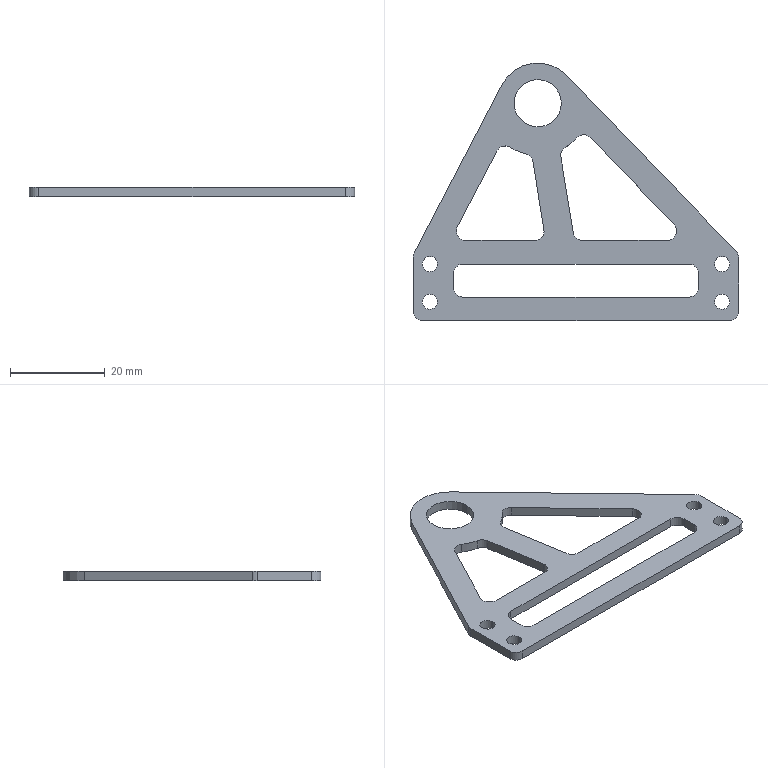Part | SolidWorks | features Fillet 6, ICE 5, Extrusion 1 | 1 solid | 47 faces | box 68.8 x 54.5 x 2 mm | volume 2944 mm3 | cylinder 30 | plane 17 | commonest cylinder face diameters 4 x17 3.2 x8 10 x2 22 x2 17 x1
STEP:
#1=CARTESIAN_POINT('',(-17.204,-27.,2.));
#2=VERTEX_POINT('',#1);
#3=CARTESIAN_POINT('',(-16.977,-26.075,2.));
#4=VERTEX_POINT('',#3);
#5=CARTESIAN_POINT('',(-15.204,-27.,2.));
#6=DIRECTION('',(0.,0.,-1.));
#7=DIRECTION('',(1.,0.,0.));
#8=AXIS2_PLACEMENT_3D('',#5,#6,#7);
#9=CIRCLE('',#8,2.);
#10=EDGE_CURVE('',#2,#4,#9,.T.);
#11=ORIENTED_EDGE('',*,*,#10,.F.);
#12=CARTESIAN_POINT('',(-17.204,-27.,0.));
#13=VERTEX_POINT('',#12);
#14=CARTESIAN_POINT('',(-17.204,-27.,0.));
#15=DIRECTION('',(0.,0.,-1.));
#16=VECTOR('',#15,1000.);
#17=LINE('',#14,#16);
#18=EDGE_CURVE('',#2,#13,#17,.T.);
#19=ORIENTED_EDGE('',*,*,#18,.T.);
#20=CARTESIAN_POINT('',(-16.977,-26.075,0.));
#21=VERTEX_POINT('',#20);
#22=CARTESIAN_POINT('',(-15.204,-27.,0.));
#23=DIRECTION('',(0.,0.,1.));
#24=DIRECTION('',(1.,0.,0.));
#25=AXIS2_PLACEMENT_3D('',#22,#23,#24);
#26=CIRCLE('',#25,2.);
#27=EDGE_CURVE('',#21,#13,#26,.T.);
#28=ORIENTED_EDGE('',*,*,#27,.F.);
#29=CARTESIAN_POINT('',(-16.977,-26.075,0.));
#30=DIRECTION('',(0.,0.,-1.));
#31=VECTOR('',#30,1000.);
#32=LINE('',#29,#31);
#33=EDGE_CURVE('',#4,#21,#32,.T.);
#34=ORIENTED_EDGE('',*,*,#33,.F.);
#35=EDGE_LOOP('',(#11,#19,#28,#34));
#36=FACE_OUTER_BOUND('',#35,.T.);
#37=CARTESIAN_POINT('',(-15.204,-27.,0.));
#38=DIRECTION('',(0.,0.,-1.));
#39=DIRECTION('',(-1.,0.,0.));
#40=AXIS2_PLACEMENT_3D('',#37,#38,#39);
#41=CYLINDRICAL_SURFACE('',#40,2.);
#42=ADVANCED_FACE('',(#36),#41,.F.);
#43=CARTESIAN_POINT('',(37.4,-34.,2.));
#44=VERTEX_POINT('',#43);
#45=CARTESIAN_POINT('',(40.6,-34.,2.));
#46=VERTEX_POINT('',#45);
#47=CARTESIAN_POINT('',(39.,-34.,2.));
#48=DIRECTION('',(0.,0.,1.));
#49=DIRECTION('',(-1.,0.,0.));
#50=AXIS2_PLACEMENT_3D('',#47,#48,#49);
#51=CIRCLE('',#50,1.6);
#52=EDGE_CURVE('',#44,#46,#51,.T.);
#53=ORIENTED_EDGE('',*,*,#52,.T.);
#54=CARTESIAN_POINT('',(40.6,-34.,0.));
#55=VERTEX_POINT('',#54);
#56=CARTESIAN_POINT('',(40.6,-34.,2.));
#57=DIRECTION('',(0.,0.,-1.));
#58=VECTOR('',#57,1000.);
#59=LINE('',#56,#58);
#60=EDGE_CURVE('',#46,#55,#59,.T.);
#61=ORIENTED_EDGE('',*,*,#60,.T.);
#62=CARTESIAN_POINT('',(37.4,-34.,0.));
#63=VERTEX_POINT('',#62);
#64=CARTESIAN_POINT('',(39.,-34.,0.));
#65=DIRECTION('',(0.,0.,1.));
#66=DIRECTION('',(-1.,0.,0.));
#67=AXIS2_PLACEMENT_3D('',#64,#65,#66);
#68=CIRCLE('',#67,1.6);
#69=EDGE_CURVE('',#63,#55,#68,.T.);
#70=ORIENTED_EDGE('',*,*,#69,.F.);
#71=CARTESIAN_POINT('',(37.4,-34.,2.));
#72=DIRECTION('',(0.,0.,-1.));
#73=VECTOR('',#72,1000.);
#74=LINE('',#71,#73);
#75=EDGE_CURVE('',#44,#63,#74,.T.);
#76=ORIENTED_EDGE('',*,*,#75,.F.);
#77=EDGE_LOOP('',(#53,#61,#70,#76));
#78=FACE_OUTER_BOUND('',#77,.T.);
#79=CARTESIAN_POINT('',(39.,-34.,2.));
#80=DIRECTION('',(0.,0.,-1.));
#81=DIRECTION('',(-1.,0.,0.));
#82=AXIS2_PLACEMENT_3D('',#79,#80,#81);
#83=CYLINDRICAL_SURFACE('',#82,1.6);
#84=ADVANCED_FACE('',(#78),#83,.F.);
#85=CARTESIAN_POINT('',(37.4,-42.,2.));
#86=VERTEX_POINT('',#85);
#87=CARTESIAN_POINT('',(40.6,-42.,2.));
#88=VERTEX_POINT('',#87);
#89=CARTESIAN_POINT('',(39.,-42.,2.));
#90=DIRECTION('',(0.,0.,1.));
#91=DIRECTION('',(-1.,0.,0.));
#92=AXIS2_PLACEMENT_3D('',#89,#90,#91);
#93=CIRCLE('',#92,1.6);
#94=EDGE_CURVE('',#86,#88,#93,.T.);
#95=ORIENTED_EDGE('',*,*,#94,.T.);
#96=CARTESIAN_POINT('',(40.6,-42.,0.));
#97=VERTEX_POINT('',#96);
#98=CARTESIAN_POINT('',(40.6,-42.,2.));
#99=DIRECTION('',(0.,0.,-1.));
#100=VECTOR('',#99,1000.);
#101=LINE('',#98,#100);
#102=EDGE_CURVE('',#88,#97,#101,.T.);
#103=ORIENTED_EDGE('',*,*,#102,.T.);
#104=CARTESIAN_POINT('',(37.4,-42.,0.));
#105=VERTEX_POINT('',#104);
#106=CARTESIAN_POINT('',(39.,-42.,0.));
#107=DIRECTION('',(0.,0.,1.));
#108=DIRECTION('',(-1.,0.,0.));
#109=AXIS2_PLACEMENT_3D('',#106,#107,#108);
#110=CIRCLE('',#109,1.6);
#111=EDGE_CURVE('',#105,#97,#110,.T.);
#112=ORIENTED_EDGE('',*,*,#111,.F.);
#113=CARTESIAN_POINT('',(37.4,-42.,2.));
#114=DIRECTION('',(0.,0.,-1.));
#115=VECTOR('',#114,1000.);
#116=LINE('',#113,#115);
#117=EDGE_CURVE('',#86,#105,#116,.T.);
#118=ORIENTED_EDGE('',*,*,#117,.F.);
#119=EDGE_LOOP('',(#95,#103,#112,#118));
#120=FACE_OUTER_BOUND('',#119,.T.);
#121=CARTESIAN_POINT('',(39.,-42.,2.));
#122=DIRECTION('',(0.,0.,-1.));
#123=DIRECTION('',(-1.,0.,0.));
#124=AXIS2_PLACEMENT_3D('',#121,#122,#123);
#125=CYLINDRICAL_SURFACE('',#124,1.6);
#126=ADVANCED_FACE('',(#120),#125,.F.);
#127=CARTESIAN_POINT('',(-24.4,-34.,2.));
#128=VERTEX_POINT('',#127);
#129=CARTESIAN_POINT('',(-21.2,-34.,2.));
#130=VERTEX_POINT('',#129);
#131=CARTESIAN_POINT('',(-22.8,-34.,2.));
#132=DIRECTION('',(0.,0.,1.));
#133=DIRECTION('',(1.,0.,0.));
#134=AXIS2_PLACEMENT_3D('',#131,#132,#133);
#135=CIRCLE('',#134,1.6);
#136=EDGE_CURVE('',#128,#130,#135,.T.);
#137=ORIENTED_EDGE('',*,*,#136,.T.);
#138=CARTESIAN_POINT('',(-21.2,-34.,0.));
#139=VERTEX_POINT('',#138);
#140=CARTESIAN_POINT('',(-21.2,-34.,2.));
#141=DIRECTION('',(0.,0.,-1.));
#142=VECTOR('',#141,1000.);
#143=LINE('',#140,#142);
#144=EDGE_CURVE('',#130,#139,#143,.T.);
#145=ORIENTED_EDGE('',*,*,#144,.T.);
#146=CARTESIAN_POINT('',(-24.4,-34.,0.));
#147=VERTEX_POINT('',#146);
#148=CARTESIAN_POINT('',(-22.8,-34.,0.));
#149=DIRECTION('',(0.,0.,1.));
#150=DIRECTION('',(1.,0.,0.));
#151=AXIS2_PLACEMENT_3D('',#148,#149,#150);
#152=CIRCLE('',#151,1.6);
#153=EDGE_CURVE('',#147,#139,#152,.T.);
#154=ORIENTED_EDGE('',*,*,#153,.F.);
#155=CARTESIAN_POINT('',(-24.4,-34.,2.));
#156=DIRECTION('',(0.,0.,-1.));
#157=VECTOR('',#156,1000.);
#158=LINE('',#155,#157);
#159=EDGE_CURVE('',#128,#147,#158,.T.);
#160=ORIENTED_EDGE('',*,*,#159,.F.);
#161=EDGE_LOOP('',(#137,#145,#154,#160));
#162=FACE_OUTER_BOUND('',#161,.T.);
#163=CARTESIAN_POINT('',(-22.8,-34.,2.));
#164=DIRECTION('',(0.,0.,-1.));
#165=DIRECTION('',(-1.,0.,0.));
#166=AXIS2_PLACEMENT_3D('',#163,#164,#165);
#167=CYLINDRICAL_SURFACE('',#166,1.6);
#168=ADVANCED_FACE('',(#162),#167,.F.);
#169=CARTESIAN_POINT('',(-24.4,-42.,2.));
#170=VERTEX_POINT('',#169);
#171=CARTESIAN_POINT('',(-21.2,-42.,2.));
#172=VERTEX_POINT('',#171);
#173=CARTESIAN_POINT('',(-22.8,-42.,2.));
#174=DIRECTION('',(0.,0.,1.));
#175=DIRECTION('',(1.,0.,0.));
#176=AXIS2_PLACEMENT_3D('',#173,#174,#175);
#177=CIRCLE('',#176,1.6);
#178=EDGE_CURVE('',#170,#172,#177,.T.);
#179=ORIENTED_EDGE('',*,*,#178,.T.);
#180=CARTESIAN_POINT('',(-21.2,-42.,0.));
#181=VERTEX_POINT('',#180);
#182=CARTESIAN_POINT('',(-21.2,-42.,2.));
#183=DIRECTION('',(0.,0.,-1.));
#184=VECTOR('',#183,1000.);
#185=LINE('',#182,#184);
#186=EDGE_CURVE('',#172,#181,#185,.T.);
#187=ORIENTED_EDGE('',*,*,#186,.T.);
#188=CARTESIAN_POINT('',(-24.4,-42.,0.));
#189=VERTEX_POINT('',#188);
#190=CARTESIAN_POINT('',(-22.8,-42.,0.));
#191=DIRECTION('',(0.,0.,1.));
#192=DIRECTION('',(1.,0.,0.));
#193=AXIS2_PLACEMENT_3D('',#190,#191,#192);
#194=CIRCLE('',#193,1.6);
#195=EDGE_CURVE('',#189,#181,#194,.T.);
#196=ORIENTED_EDGE('',*,*,#195,.F.);
#197=CARTESIAN_POINT('',(-24.4,-42.,2.));
#198=DIRECTION('',(0.,0.,-1.));
#199=VECTOR('',#198,1000.);
#200=LINE('',#197,#199);
#201=EDGE_CURVE('',#170,#189,#200,.T.);
#202=ORIENTED_EDGE('',*,*,#201,.F.);
#203=EDGE_LOOP('',(#179,#187,#196,#202));
#204=FACE_OUTER_BOUND('',#203,.T.);
#205=CARTESIAN_POINT('',(-22.8,-42.,2.));
#206=DIRECTION('',(0.,0.,-1.));
#207=DIRECTION('',(-1.,0.,0.));
#208=AXIS2_PLACEMENT_3D('',#205,#206,#207);
#209=CYLINDRICAL_SURFACE('',#208,1.6);
#210=ADVANCED_FACE('',(#204),#209,.F.);
#211=CARTESIAN_POINT('',(-5.,0.,2.));
#212=VERTEX_POINT('',#211);
#213=CARTESIAN_POINT('',(5.,0.,2.));
#214=VERTEX_POINT('',#213);
#215=CARTESIAN_POINT('',(0.,0.,2.));
#216=DIRECTION('',(0.,0.,1.));
#217=DIRECTION('',(1.,0.,0.));
#218=AXIS2_PLACEMENT_3D('',#215,#216,#217);
#219=CIRCLE('',#218,5.);
#220=EDGE_CURVE('',#212,#214,#219,.T.);
#221=ORIENTED_EDGE('',*,*,#220,.T.);
#222=CARTESIAN_POINT('',(5.,0.,0.));
#223=VERTEX_POINT('',#222);
#224=CARTESIAN_POINT('',(5.,0.,2.));
#225=DIRECTION('',(0.,0.,-1.));
#226=VECTOR('',#225,1000.);
#227=LINE('',#224,#226);
#228=EDGE_CURVE('',#214,#223,#227,.T.);
#229=ORIENTED_EDGE('',*,*,#228,.T.);
#230=CARTESIAN_POINT('',(-5.,0.,0.));
#231=VERTEX_POINT('',#230);
#232=CARTESIAN_POINT('',(0.,0.,0.));
#233=DIRECTION('',(0.,0.,1.));
#234=DIRECTION('',(1.,0.,0.));
#235=AXIS2_PLACEMENT_3D('',#232,#233,#234);
#236=CIRCLE('',#235,5.);
#237=EDGE_CURVE('',#231,#223,#236,.T.);
#238=ORIENTED_EDGE('',*,*,#237,.F.);
#239=CARTESIAN_POINT('',(-5.,0.,2.));
#240=DIRECTION('',(0.,0.,-1.));
#241=VECTOR('',#240,1000.);
#242=LINE('',#239,#241);
#243=EDGE_CURVE('',#212,#231,#242,.T.);
#244=ORIENTED_EDGE('',*,*,#243,.F.);
#245=EDGE_LOOP('',(#221,#229,#238,#244));
#246=FACE_OUTER_BOUND('',#245,.T.);
#247=CARTESIAN_POINT('',(0.,0.,2.));
#248=DIRECTION('',(0.,0.,-1.));
#249=DIRECTION('',(-1.,0.,0.));
#250=AXIS2_PLACEMENT_3D('',#247,#248,#249);
#251=CYLINDRICAL_SURFACE('',#250,5.);
#252=ADVANCED_FACE('',(#246),#251,.F.);
#253=CARTESIAN_POINT('',(-17.8,-36.,2.));
#254=VERTEX_POINT('',#253);
#255=CARTESIAN_POINT('',(-17.8,-39.,2.));
#256=VERTEX_POINT('',#255);
#257=CARTESIAN_POINT('',(-17.8,-34.,2.));
#258=DIRECTION('',(0.,-1.,0.));
#259=VECTOR('',#258,1000.);
#260=LINE('',#257,#259);
#261=EDGE_CURVE('',#254,#256,#260,.T.);
#262=ORIENTED_EDGE('',*,*,#261,.F.);
#263=CARTESIAN_POINT('',(-15.8,-34.,2.));
#264=VERTEX_POINT('',#263);
#265=CARTESIAN_POINT('',(-15.8,-36.,2.));
#266=DIRECTION('',(0.,0.,-1.));
#267=DIRECTION('',(1.,0.,0.));
#268=AXIS2_PLACEMENT_3D('',#265,#266,#267);
#269=CIRCLE('',#268,2.);
#270=EDGE_CURVE('',#254,#264,#269,.T.);
#271=ORIENTED_EDGE('',*,*,#270,.T.);
#272=CARTESIAN_POINT('',(32.,-34.,2.));
#273=VERTEX_POINT('',#272);
#274=CARTESIAN_POINT('',(-17.8,-34.,2.));
#275=DIRECTION('',(-1.,0.,0.));
#276=VECTOR('',#275,1000.);
#277=LINE('',#274,#276);
#278=EDGE_CURVE('',#273,#264,#277,.T.);
#279=ORIENTED_EDGE('',*,*,#278,.F.);
#280=CARTESIAN_POINT('',(34.,-36.,2.));
#281=VERTEX_POINT('',#280);
#282=CARTESIAN_POINT('',(32.,-36.,2.));
#283=DIRECTION('',(0.,0.,-1.));
#284=DIRECTION('',(1.,0.,0.));
#285=AXIS2_PLACEMENT_3D('',#282,#283,#284);
#286=CIRCLE('',#285,2.);
#287=EDGE_CURVE('',#273,#281,#286,.T.);
#288=ORIENTED_EDGE('',*,*,#287,.T.);
#289=CARTESIAN_POINT('',(34.,-39.,2.));
#290=VERTEX_POINT('',#289);
#291=CARTESIAN_POINT('',(34.,-34.,2.));
#292=DIRECTION('',(0.,1.,0.));
#293=VECTOR('',#292,1000.);
#294=LINE('',#291,#293);
#295=EDGE_CURVE('',#290,#281,#294,.T.);
#296=ORIENTED_EDGE('',*,*,#295,.F.);
#297=CARTESIAN_POINT('',(32.,-41.,2.));
#298=VERTEX_POINT('',#297);
#299=CARTESIAN_POINT('',(32.,-39.,2.));
#300=DIRECTION('',(0.,0.,-1.));
#301=DIRECTION('',(1.,0.,0.));
#302=AXIS2_PLACEMENT_3D('',#299,#300,#301);
#303=CIRCLE('',#302,2.);
#304=EDGE_CURVE('',#290,#298,#303,.T.);
#305=ORIENTED_EDGE('',*,*,#304,.T.);
#306=CARTESIAN_POINT('',(-15.8,-41.,2.));
#307=VERTEX_POINT('',#306);
#308=CARTESIAN_POINT('',(-17.8,-41.,2.));
#309=DIRECTION('',(1.,0.,0.));
#310=VECTOR('',#309,1000.);
#311=LINE('',#308,#310);
#312=EDGE_CURVE('',#307,#298,#311,.T.);
#313=ORIENTED_EDGE('',*,*,#312,.F.);
#314=CARTESIAN_POINT('',(-15.8,-39.,2.));
#315=DIRECTION('',(0.,0.,-1.));
#316=DIRECTION('',(1.,0.,0.));
#317=AXIS2_PLACEMENT_3D('',#314,#315,#316);
#318=CIRCLE('',#317,2.);
#319=EDGE_CURVE('',#307,#256,#318,.T.);
#320=ORIENTED_EDGE('',*,*,#319,.T.);
#321=EDGE_LOOP('',(#262,#271,#279,#288,#296,#305,#313,#320));
#322=FACE_BOUND('',#321,.T.);
#323=CARTESIAN_POINT('',(8.218,-7.312,2.));
#324=VERTEX_POINT('',#323);
#325=CARTESIAN_POINT('',(5.813,-9.338,2.));
#326=VERTEX_POINT('',#325);
#327=CARTESIAN_POINT('',(0.,0.,2.));
#328=DIRECTION('',(0.,0.,-1.));
#329=DIRECTION('',(1.,0.,0.));
#330=AXIS2_PLACEMENT_3D('',#327,#328,#329);
#331=CIRCLE('',#330,11.);
#332=EDGE_CURVE('',#324,#326,#331,.T.);
#333=ORIENTED_EDGE('',*,*,#332,.F.);
#334=CARTESIAN_POINT('',(11.153,-7.254,2.));
#335=VERTEX_POINT('',#334);
#336=CARTESIAN_POINT('',(9.712,-8.641,2.));
#337=DIRECTION('',(0.,0.,-1.));
#338=DIRECTION('',(1.,0.,0.));
#339=AXIS2_PLACEMENT_3D('',#336,#337,#338);
#340=CIRCLE('',#339,2.);
#341=EDGE_CURVE('',#324,#335,#340,.T.);
#342=ORIENTED_EDGE('',*,*,#341,.T.);
#343=CARTESIAN_POINT('',(28.838,-25.612,2.));
#344=VERTEX_POINT('',#343);
#345=CARTESIAN_POINT('',(32.101,-29.,2.));
#346=DIRECTION('',(-0.6938,0.7202,0.));
#347=VECTOR('',#346,1000.);
#348=LINE('',#345,#347);
#349=EDGE_CURVE('',#344,#335,#348,.T.);
#350=ORIENTED_EDGE('',*,*,#349,.F.);
#351=CARTESIAN_POINT('',(27.397,-29.,2.));
#352=VERTEX_POINT('',#351);
#353=CARTESIAN_POINT('',(27.397,-27.,2.));
#354=DIRECTION('',(0.,0.,-1.));
#355=DIRECTION('',(1.,0.,0.));
#356=AXIS2_PLACEMENT_3D('',#353,#354,#355);
#357=CIRCLE('',#356,2.);
#358=EDGE_CURVE('',#344,#352,#357,.T.);
#359=ORIENTED_EDGE('',*,*,#358,.T.);
#360=CARTESIAN_POINT('',(9.479,-29.,2.));
#361=VERTEX_POINT('',#360);
#362=CARTESIAN_POINT('',(7.78,-29.,2.));
#363=DIRECTION('',(1.,0.,0.));
#364=VECTOR('',#363,1000.);
#365=LINE('',#362,#364);
#366=EDGE_CURVE('',#361,#352,#365,.T.);
#367=ORIENTED_EDGE('',*,*,#366,.F.);
#368=CARTESIAN_POINT('',(7.505,-27.323,2.));
#369=VERTEX_POINT('',#368);
#370=CARTESIAN_POINT('',(9.479,-27.,2.));
#371=DIRECTION('',(0.,0.,-1.));
#372=DIRECTION('',(1.,0.,0.));
#373=AXIS2_PLACEMENT_3D('',#370,#371,#372);
#374=CIRCLE('',#373,2.);
#375=EDGE_CURVE('',#361,#369,#374,.T.);
#376=ORIENTED_EDGE('',*,*,#375,.T.);
#377=CARTESIAN_POINT('',(4.896,-11.359,2.));
#378=VERTEX_POINT('',#377);
#379=CARTESIAN_POINT('',(4.668,-9.961,2.));
#380=DIRECTION('',(0.1613,-0.9869,0.));
#381=VECTOR('',#380,1000.);
#382=LINE('',#379,#381);
#383=EDGE_CURVE('',#378,#369,#382,.T.);
#384=ORIENTED_EDGE('',*,*,#383,.F.);
#385=CARTESIAN_POINT('',(6.87,-11.036,2.));
#386=DIRECTION('',(0.,0.,-1.));
#387=DIRECTION('',(1.,0.,0.));
#388=AXIS2_PLACEMENT_3D('',#385,#386,#387);
#389=CIRCLE('',#388,2.);
#390=EDGE_CURVE('',#378,#326,#389,.T.);
#391=ORIENTED_EDGE('',*,*,#390,.T.);
#392=EDGE_LOOP('',(#333,#342,#350,#359,#367,#376,#384,#391));
#393=FACE_BOUND('',#392,.T.);
#394=CARTESIAN_POINT('',(-2.538,-10.703,2.));
#395=VERTEX_POINT('',#394);
#396=CARTESIAN_POINT('',(-5.82,-9.334,2.));
#397=VERTEX_POINT('',#396);
#398=CARTESIAN_POINT('',(0.,0.,2.));
#399=DIRECTION('',(0.,0.,-1.));
#400=DIRECTION('',(1.,0.,0.));
#401=AXIS2_PLACEMENT_3D('',#398,#399,#400);
#402=CIRCLE('',#401,11.);
#403=EDGE_CURVE('',#395,#397,#402,.T.);
#404=ORIENTED_EDGE('',*,*,#403,.F.);
#405=CARTESIAN_POINT('',(-1.025,-12.327,2.));
#406=VERTEX_POINT('',#405);
#407=CARTESIAN_POINT('',(-2.999,-12.649,2.));
#408=DIRECTION('',(0.,0.,-1.));
#409=DIRECTION('',(1.,0.,0.));
#410=AXIS2_PLACEMENT_3D('',#407,#408,#409);
#411=CIRCLE('',#410,2.);
#412=EDGE_CURVE('',#395,#406,#411,.T.);
#413=ORIENTED_EDGE('',*,*,#412,.T.);
#414=CARTESIAN_POINT('',(1.32,-26.677,2.));
#415=VERTEX_POINT('',#414);
#416=CARTESIAN_POINT('',(1.7,-29.,2.));
#417=DIRECTION('',(-0.1613,0.9869,0.));
#418=VECTOR('',#417,1000.);
#419=LINE('',#416,#418);
#420=EDGE_CURVE('',#415,#406,#419,.T.);
#421=ORIENTED_EDGE('',*,*,#420,.F.);
#422=CARTESIAN_POINT('',(-0.6534,-29.,2.));
#423=VERTEX_POINT('',#422);
#424=CARTESIAN_POINT('',(-0.6534,-27.,2.));
#425=DIRECTION('',(0.,0.,-1.));
#426=DIRECTION('',(1.,0.,0.));
#427=AXIS2_PLACEMENT_3D('',#424,#425,#426);
#428=CIRCLE('',#427,2.);
#429=EDGE_CURVE('',#415,#423,#428,.T.);
#430=ORIENTED_EDGE('',*,*,#429,.T.);
#431=CARTESIAN_POINT('',(-15.204,-29.,2.));
#432=VERTEX_POINT('',#431);
#433=CARTESIAN_POINT('',(-18.502,-29.,2.));
#434=DIRECTION('',(1.,0.,0.));
#435=VECTOR('',#434,1000.);
#436=LINE('',#433,#435);
#437=EDGE_CURVE('',#432,#423,#436,.T.);
#438=ORIENTED_EDGE('',*,*,#437,.F.);
#439=CARTESIAN_POINT('',(-15.204,-27.,2.));
#440=DIRECTION('',(0.,0.,-1.));
#441=DIRECTION('',(1.,0.,0.));
#442=AXIS2_PLACEMENT_3D('',#439,#440,#441);
#443=CIRCLE('',#442,2.);
#444=EDGE_CURVE('',#432,#2,#443,.T.);
#445=ORIENTED_EDGE('',*,*,#444,.T.);
#446=ORIENTED_EDGE('',*,*,#10,.T.);
#447=CARTESIAN_POINT('',(-8.652,-10.107,2.));
#448=VERTEX_POINT('',#447);
#449=CARTESIAN_POINT('',(-7.553,-7.997,2.));
#450=DIRECTION('',(-0.4623,-0.8867,0.));
#451=VECTOR('',#450,1000.);
#452=LINE('',#449,#451);
#453=EDGE_CURVE('',#448,#4,#452,.T.);
#454=ORIENTED_EDGE('',*,*,#453,.F.);
#455=CARTESIAN_POINT('',(-6.879,-11.031,2.));
#456=DIRECTION('',(0.,0.,-1.));
#457=DIRECTION('',(1.,0.,0.));
#458=AXIS2_PLACEMENT_3D('',#455,#456,#457);
#459=CIRCLE('',#458,2.);
#460=EDGE_CURVE('',#448,#397,#459,.T.);
#461=ORIENTED_EDGE('',*,*,#460,.T.);
#462=EDGE_LOOP('',(#404,#413,#421,#430,#438,#445,#446,#454,#461));
#463=FACE_BOUND('',#462,.T.);
#464=ORIENTED_EDGE('',*,*,#94,.F.);
#465=CARTESIAN_POINT('',(39.,-42.,2.));
#466=DIRECTION('',(0.,0.,1.));
#467=DIRECTION('',(-1.,0.,0.));
#468=AXIS2_PLACEMENT_3D('',#465,#466,#467);
#469=CIRCLE('',#468,1.6);
#470=EDGE_CURVE('',#88,#86,#469,.T.);
#471=ORIENTED_EDGE('',*,*,#470,.F.);
#472=EDGE_LOOP('',(#464,#471));
#473=FACE_BOUND('',#472,.T.);
#474=ORIENTED_EDGE('',*,*,#178,.F.);
#475=CARTESIAN_POINT('',(-22.8,-42.,2.));
#476=DIRECTION('',(0.,0.,1.));
#477=DIRECTION('',(1.,0.,0.));
#478=AXIS2_PLACEMENT_3D('',#475,#476,#477);
#479=CIRCLE('',#478,1.6);
#480=EDGE_CURVE('',#172,#170,#479,.T.);
#481=ORIENTED_EDGE('',*,*,#480,.F.);
#482=EDGE_LOOP('',(#474,#481));
#483=FACE_BOUND('',#482,.T.);
#484=CARTESIAN_POINT('',(42.5,-44.,2.));
#485=VERTEX_POINT('',#484);
#486=CARTESIAN_POINT('',(42.5,-32.674,2.));
#487=VERTEX_POINT('',#486);
#488=CARTESIAN_POINT('',(42.5,-46.,2.));
#489=DIRECTION('',(0.,1.,0.));
#490=VECTOR('',#489,1000.);
#491=LINE('',#488,#490);
#492=EDGE_CURVE('',#485,#487,#491,.T.);
#493=ORIENTED_EDGE('',*,*,#492,.T.);
#494=CARTESIAN_POINT('',(41.94,-31.287,2.));
#495=VERTEX_POINT('',#494);
#496=CARTESIAN_POINT('',(40.5,-32.674,2.));
#497=DIRECTION('',(0.,0.,1.));
#498=DIRECTION('',(1.,0.,0.));
#499=AXIS2_PLACEMENT_3D('',#496,#497,#498);
#500=CIRCLE('',#499,2.);
#501=EDGE_CURVE('',#487,#495,#500,.T.);
#502=ORIENTED_EDGE('',*,*,#501,.T.);
#503=CARTESIAN_POINT('',(6.122,5.897,2.));
#504=VERTEX_POINT('',#503);
#505=CARTESIAN_POINT('',(42.5,-31.868,2.));
#506=DIRECTION('',(-0.6938,0.7202,0.));
#507=VECTOR('',#506,1000.);
#508=LINE('',#505,#507);
#509=EDGE_CURVE('',#495,#504,#508,.T.);
#510=ORIENTED_EDGE('',*,*,#509,.T.);
#511=CARTESIAN_POINT('',(-7.537,3.929,2.));
#512=VERTEX_POINT('',#511);
#513=CARTESIAN_POINT('',(0.,0.,2.));
#514=DIRECTION('',(0.,0.,1.));
#515=DIRECTION('',(1.,0.,0.));
#516=AXIS2_PLACEMENT_3D('',#513,#514,#515);
#517=CIRCLE('',#516,8.5);
#518=EDGE_CURVE('',#504,#512,#517,.T.);
#519=ORIENTED_EDGE('',*,*,#518,.T.);
#520=CARTESIAN_POINT('',(-26.073,-31.626,2.));
#521=VERTEX_POINT('',#520);
#522=CARTESIAN_POINT('',(-7.537,3.929,2.));
#523=DIRECTION('',(-0.4623,-0.8867,0.));
#524=VECTOR('',#523,1000.);
#525=LINE('',#522,#524);
#526=EDGE_CURVE('',#512,#521,#525,.T.);
#527=ORIENTED_EDGE('',*,*,#526,.T.);
#528=CARTESIAN_POINT('',(-26.3,-32.551,2.));
#529=VERTEX_POINT('',#528);
#530=CARTESIAN_POINT('',(-24.3,-32.551,2.));
#531=DIRECTION('',(0.,0.,1.));
#532=DIRECTION('',(1.,0.,0.));
#533=AXIS2_PLACEMENT_3D('',#530,#531,#532);
#534=CIRCLE('',#533,2.);
#535=EDGE_CURVE('',#521,#529,#534,.T.);
#536=ORIENTED_EDGE('',*,*,#535,.T.);
#537=CARTESIAN_POINT('',(-26.3,-44.,2.));
#538=VERTEX_POINT('',#537);
#539=CARTESIAN_POINT('',(-26.3,-32.061,2.));
#540=DIRECTION('',(0.,-1.,0.));
#541=VECTOR('',#540,1000.);
#542=LINE('',#539,#541);
#543=EDGE_CURVE('',#529,#538,#542,.T.);
#544=ORIENTED_EDGE('',*,*,#543,.T.);
#545=CARTESIAN_POINT('',(-24.3,-46.,2.));
#546=VERTEX_POINT('',#545);
#547=CARTESIAN_POINT('',(-24.3,-44.,2.));
#548=DIRECTION('',(0.,0.,1.));
#549=DIRECTION('',(1.,0.,0.));
#550=AXIS2_PLACEMENT_3D('',#547,#548,#549);
#551=CIRCLE('',#550,2.);
#552=EDGE_CURVE('',#538,#546,#551,.T.);
#553=ORIENTED_EDGE('',*,*,#552,.T.);
#554=CARTESIAN_POINT('',(40.5,-46.,2.));
#555=VERTEX_POINT('',#554);
#556=CARTESIAN_POINT('',(-26.3,-46.,2.));
#557=DIRECTION('',(1.,0.,0.));
#558=VECTOR('',#557,1000.);
#559=LINE('',#556,#558);
#560=EDGE_CURVE('',#546,#555,#559,.T.);
#561=ORIENTED_EDGE('',*,*,#560,.T.);
#562=CARTESIAN_POINT('',(40.5,-44.,2.));
#563=DIRECTION('',(0.,0.,1.));
#564=DIRECTION('',(1.,0.,0.));
#565=AXIS2_PLACEMENT_3D('',#562,#563,#564);
#566=CIRCLE('',#565,2.);
#567=EDGE_CURVE('',#555,#485,#566,.T.);
#568=ORIENTED_EDGE('',*,*,#567,.T.);
#569=EDGE_LOOP('',(#493,#502,#510,#519,#527,#536,#544,#553,#561,#568));
#570=FACE_OUTER_BOUND('',#569,.T.);
#571=ORIENTED_EDGE('',*,*,#220,.F.);
#572=CARTESIAN_POINT('',(0.,0.,2.));
#573=DIRECTION('',(0.,0.,1.));
#574=DIRECTION('',(1.,0.,0.));
#575=AXIS2_PLACEMENT_3D('',#572,#573,#574);
#576=CIRCLE('',#575,5.);
#577=EDGE_CURVE('',#214,#212,#576,.T.);
#578=ORIENTED_EDGE('',*,*,#577,.F.);
#579=EDGE_LOOP('',(#571,#578));
#580=FACE_BOUND('',#579,.T.);
#581=ORIENTED_EDGE('',*,*,#136,.F.);
#582=CARTESIAN_POINT('',(-22.8,-34.,2.));
#583=DIRECTION('',(0.,0.,1.));
#584=DIRECTION('',(1.,0.,0.));
#585=AXIS2_PLACEMENT_3D('',#582,#583,#584);
#586=CIRCLE('',#585,1.6);
#587=EDGE_CURVE('',#130,#128,#586,.T.);
#588=ORIENTED_EDGE('',*,*,#587,.F.);
#589=EDGE_LOOP('',(#581,#588));
#590=FACE_BOUND('',#589,.T.);
#591=ORIENTED_EDGE('',*,*,#52,.F.);
#592=CARTESIAN_POINT('',(39.,-34.,2.));
#593=DIRECTION('',(0.,0.,1.));
#594=DIRECTION('',(-1.,0.,0.));
#595=AXIS2_PLACEMENT_3D('',#592,#593,#594);
#596=CIRCLE('',#595,1.6);
#597=EDGE_CURVE('',#46,#44,#596,.T.);
#598=ORIENTED_EDGE('',*,*,#597,.F.);
#599=EDGE_LOOP('',(#591,#598));
#600=FACE_BOUND('',#599,.T.);
#601=CARTESIAN_POINT('',(0.,0.,2.));
#602=DIRECTION('',(0.,0.,1.));
#603=DIRECTION('',(1.,0.,0.));
#604=AXIS2_PLACEMENT_3D('',#601,#602,#603);
#605=PLANE('',#604);
#606=ADVANCED_FACE('',(#322,#393,#463,#473,#483,#570,#580,#590,#600),#605,.T.);
#607=CARTESIAN_POINT('',(34.,-39.,0.));
#608=VERTEX_POINT('',#607);
#609=CARTESIAN_POINT('',(34.,-36.,0.));
#610=VERTEX_POINT('',#609);
#611=CARTESIAN_POINT('',(34.,-34.,0.));
#612=DIRECTION('',(0.,1.,0.));
#613=VECTOR('',#612,1000.);
#614=LINE('',#611,#613);
#615=EDGE_CURVE('',#608,#610,#614,.T.);
#616=ORIENTED_EDGE('',*,*,#615,.T.);
#617=CARTESIAN_POINT('',(32.,-34.,0.));
#618=VERTEX_POINT('',#617);
#619=CARTESIAN_POINT('',(32.,-36.,0.));
#620=DIRECTION('',(0.,0.,1.));
#621=DIRECTION('',(1.,0.,0.));
#622=AXIS2_PLACEMENT_3D('',#619,#620,#621);
#623=CIRCLE('',#622,2.);
#624=EDGE_CURVE('',#610,#618,#623,.T.);
#625=ORIENTED_EDGE('',*,*,#624,.T.);
#626=CARTESIAN_POINT('',(-15.8,-34.,0.));
#627=VERTEX_POINT('',#626);
#628=CARTESIAN_POINT('',(-17.8,-34.,0.));
#629=DIRECTION('',(-1.,0.,0.));
#630=VECTOR('',#629,1000.);
#631=LINE('',#628,#630);
#632=EDGE_CURVE('',#618,#627,#631,.T.);
#633=ORIENTED_EDGE('',*,*,#632,.T.);
#634=CARTESIAN_POINT('',(-17.8,-36.,0.));
#635=VERTEX_POINT('',#634);
#636=CARTESIAN_POINT('',(-15.8,-36.,0.));
#637=DIRECTION('',(0.,0.,1.));
#638=DIRECTION('',(1.,0.,0.));
#639=AXIS2_PLACEMENT_3D('',#636,#637,#638);
#640=CIRCLE('',#639,2.);
#641=EDGE_CURVE('',#627,#635,#640,.T.);
#642=ORIENTED_EDGE('',*,*,#641,.T.);
#643=CARTESIAN_POINT('',(-17.8,-39.,0.));
#644=VERTEX_POINT('',#643);
#645=CARTESIAN_POINT('',(-17.8,-34.,0.));
#646=DIRECTION('',(0.,-1.,0.));
#647=VECTOR('',#646,1000.);
#648=LINE('',#645,#647);
#649=EDGE_CURVE('',#635,#644,#648,.T.);
#650=ORIENTED_EDGE('',*,*,#649,.T.);
#651=CARTESIAN_POINT('',(-15.8,-41.,0.));
#652=VERTEX_POINT('',#651);
#653=CARTESIAN_POINT('',(-15.8,-39.,0.));
#654=DIRECTION('',(0.,0.,1.));
#655=DIRECTION('',(1.,0.,0.));
#656=AXIS2_PLACEMENT_3D('',#653,#654,#655);
#657=CIRCLE('',#656,2.);
#658=EDGE_CURVE('',#644,#652,#657,.T.);
#659=ORIENTED_EDGE('',*,*,#658,.T.);
#660=CARTESIAN_POINT('',(32.,-41.,0.));
#661=VERTEX_POINT('',#660);
#662=CARTESIAN_POINT('',(-17.8,-41.,0.));
#663=DIRECTION('',(1.,0.,0.));
#664=VECTOR('',#663,1000.);
#665=LINE('',#662,#664);
#666=EDGE_CURVE('',#652,#661,#665,.T.);
#667=ORIENTED_EDGE('',*,*,#666,.T.);
#668=CARTESIAN_POINT('',(32.,-39.,0.));
#669=DIRECTION('',(0.,0.,1.));
#670=DIRECTION('',(1.,0.,0.));
#671=AXIS2_PLACEMENT_3D('',#668,#669,#670);
#672=CIRCLE('',#671,2.);
#673=EDGE_CURVE('',#661,#608,#672,.T.);
#674=ORIENTED_EDGE('',*,*,#673,.T.);
#675=EDGE_LOOP('',(#616,#625,#633,#642,#650,#659,#667,#674));
#676=FACE_BOUND('',#675,.T.);
#677=CARTESIAN_POINT('',(9.479,-29.,0.));
#678=VERTEX_POINT('',#677);
#679=CARTESIAN_POINT('',(27.397,-29.,0.));
#680=VERTEX_POINT('',#679);
#681=CARTESIAN_POINT('',(7.78,-29.,0.));
#682=DIRECTION('',(1.,0.,0.));
#683=VECTOR('',#682,1000.);
#684=LINE('',#681,#683);
#685=EDGE_CURVE('',#678,#680,#684,.T.);
#686=ORIENTED_EDGE('',*,*,#685,.T.);
#687=CARTESIAN_POINT('',(28.838,-25.612,0.));
#688=VERTEX_POINT('',#687);
#689=CARTESIAN_POINT('',(27.397,-27.,0.));
#690=DIRECTION('',(0.,0.,1.));
#691=DIRECTION('',(1.,0.,0.));
#692=AXIS2_PLACEMENT_3D('',#689,#690,#691);
#693=CIRCLE('',#692,2.);
#694=EDGE_CURVE('',#680,#688,#693,.T.);
#695=ORIENTED_EDGE('',*,*,#694,.T.);
#696=CARTESIAN_POINT('',(11.153,-7.254,0.));
#697=VERTEX_POINT('',#696);
#698=CARTESIAN_POINT('',(32.101,-29.,0.));
#699=DIRECTION('',(-0.6938,0.7202,0.));
#700=VECTOR('',#699,1000.);
#701=LINE('',#698,#700);
#702=EDGE_CURVE('',#688,#697,#701,.T.);
#703=ORIENTED_EDGE('',*,*,#702,.T.);
#704=CARTESIAN_POINT('',(8.218,-7.312,0.));
#705=VERTEX_POINT('',#704);
#706=CARTESIAN_POINT('',(9.712,-8.641,0.));
#707=DIRECTION('',(0.,0.,1.));
#708=DIRECTION('',(1.,0.,0.));
#709=AXIS2_PLACEMENT_3D('',#706,#707,#708);
#710=CIRCLE('',#709,2.);
#711=EDGE_CURVE('',#697,#705,#710,.T.);
#712=ORIENTED_EDGE('',*,*,#711,.T.);
#713=CARTESIAN_POINT('',(5.813,-9.338,0.));
#714=VERTEX_POINT('',#713);
#715=CARTESIAN_POINT('',(0.,0.,0.));
#716=DIRECTION('',(0.,0.,-1.));
#717=DIRECTION('',(1.,0.,0.));
#718=AXIS2_PLACEMENT_3D('',#715,#716,#717);
#719=CIRCLE('',#718,11.);
#720=EDGE_CURVE('',#705,#714,#719,.T.);
#721=ORIENTED_EDGE('',*,*,#720,.T.);
#722=CARTESIAN_POINT('',(4.896,-11.359,0.));
#723=VERTEX_POINT('',#722);
#724=CARTESIAN_POINT('',(6.87,-11.036,0.));
#725=DIRECTION('',(0.,0.,1.));
#726=DIRECTION('',(1.,0.,0.));
#727=AXIS2_PLACEMENT_3D('',#724,#725,#726);
#728=CIRCLE('',#727,2.);
#729=EDGE_CURVE('',#714,#723,#728,.T.);
#730=ORIENTED_EDGE('',*,*,#729,.T.);
#731=CARTESIAN_POINT('',(7.505,-27.323,0.));
#732=VERTEX_POINT('',#731);
#733=CARTESIAN_POINT('',(4.668,-9.961,0.));
#734=DIRECTION('',(0.1613,-0.9869,0.));
#735=VECTOR('',#734,1000.);
#736=LINE('',#733,#735);
#737=EDGE_CURVE('',#723,#732,#736,.T.);
#738=ORIENTED_EDGE('',*,*,#737,.T.);
#739=CARTESIAN_POINT('',(9.479,-27.,0.));
#740=DIRECTION('',(0.,0.,1.));
#741=DIRECTION('',(1.,0.,0.));
#742=AXIS2_PLACEMENT_3D('',#739,#740,#741);
#743=CIRCLE('',#742,2.);
#744=EDGE_CURVE('',#732,#678,#743,.T.);
#745=ORIENTED_EDGE('',*,*,#744,.T.);
#746=EDGE_LOOP('',(#686,#695,#703,#712,#721,#730,#738,#745));
#747=FACE_BOUND('',#746,.T.);
#748=CARTESIAN_POINT('',(-15.204,-29.,0.));
#749=VERTEX_POINT('',#748);
#750=CARTESIAN_POINT('',(-0.6534,-29.,0.));
#751=VERTEX_POINT('',#750);
#752=CARTESIAN_POINT('',(-18.502,-29.,0.));
#753=DIRECTION('',(1.,0.,0.));
#754=VECTOR('',#753,1000.);
#755=LINE('',#752,#754);
#756=EDGE_CURVE('',#749,#751,#755,.T.);
#757=ORIENTED_EDGE('',*,*,#756,.T.);
#758=CARTESIAN_POINT('',(1.32,-26.677,0.));
#759=VERTEX_POINT('',#758);
#760=CARTESIAN_POINT('',(-0.6534,-27.,0.));
#761=DIRECTION('',(0.,0.,1.));
#762=DIRECTION('',(1.,0.,0.));
#763=AXIS2_PLACEMENT_3D('',#760,#761,#762);
#764=CIRCLE('',#763,2.);
#765=EDGE_CURVE('',#751,#759,#764,.T.);
#766=ORIENTED_EDGE('',*,*,#765,.T.);
#767=CARTESIAN_POINT('',(-1.025,-12.327,0.));
#768=VERTEX_POINT('',#767);
#769=CARTESIAN_POINT('',(1.7,-29.,0.));
#770=DIRECTION('',(-0.1613,0.9869,0.));
#771=VECTOR('',#770,1000.);
#772=LINE('',#769,#771);
#773=EDGE_CURVE('',#759,#768,#772,.T.);
#774=ORIENTED_EDGE('',*,*,#773,.T.);
#775=CARTESIAN_POINT('',(-2.538,-10.703,0.));
#776=VERTEX_POINT('',#775);
#777=CARTESIAN_POINT('',(-2.999,-12.649,0.));
#778=DIRECTION('',(0.,0.,1.));
#779=DIRECTION('',(1.,0.,0.));
#780=AXIS2_PLACEMENT_3D('',#777,#778,#779);
#781=CIRCLE('',#780,2.);
#782=EDGE_CURVE('',#768,#776,#781,.T.);
#783=ORIENTED_EDGE('',*,*,#782,.T.);
#784=CARTESIAN_POINT('',(-5.82,-9.334,0.));
#785=VERTEX_POINT('',#784);
#786=CARTESIAN_POINT('',(0.,0.,0.));
#787=DIRECTION('',(0.,0.,-1.));
#788=DIRECTION('',(1.,0.,0.));
#789=AXIS2_PLACEMENT_3D('',#786,#787,#788);
#790=CIRCLE('',#789,11.);
#791=EDGE_CURVE('',#776,#785,#790,.T.);
#792=ORIENTED_EDGE('',*,*,#791,.T.);
#793=CARTESIAN_POINT('',(-8.652,-10.107,0.));
#794=VERTEX_POINT('',#793);
#795=CARTESIAN_POINT('',(-6.879,-11.031,0.));
#796=DIRECTION('',(0.,0.,1.));
#797=DIRECTION('',(1.,0.,0.));
#798=AXIS2_PLACEMENT_3D('',#795,#796,#797);
#799=CIRCLE('',#798,2.);
#800=EDGE_CURVE('',#785,#794,#799,.T.);
#801=ORIENTED_EDGE('',*,*,#800,.T.);
#802=CARTESIAN_POINT('',(-7.553,-7.997,0.));
#803=DIRECTION('',(-0.4623,-0.8867,0.));
#804=VECTOR('',#803,1000.);
#805=LINE('',#802,#804);
#806=EDGE_CURVE('',#794,#21,#805,.T.);
#807=ORIENTED_EDGE('',*,*,#806,.T.);
#808=ORIENTED_EDGE('',*,*,#27,.T.);
#809=CARTESIAN_POINT('',(-15.204,-27.,0.));
#810=DIRECTION('',(0.,0.,1.));
#811=DIRECTION('',(1.,0.,0.));
#812=AXIS2_PLACEMENT_3D('',#809,#810,#811);
#813=CIRCLE('',#812,2.);
#814=EDGE_CURVE('',#13,#749,#813,.T.);
#815=ORIENTED_EDGE('',*,*,#814,.T.);
#816=EDGE_LOOP('',(#757,#766,#774,#783,#792,#801,#807,#808,#815));
#817=FACE_BOUND('',#816,.T.);
#818=CARTESIAN_POINT('',(41.94,-31.287,0.));
#819=VERTEX_POINT('',#818);
#820=CARTESIAN_POINT('',(6.122,5.897,0.));
#821=VERTEX_POINT('',#820);
#822=CARTESIAN_POINT('',(42.5,-31.868,0.));
#823=DIRECTION('',(-0.6938,0.7202,0.));
#824=VECTOR('',#823,1000.);
#825=LINE('',#822,#824);
#826=EDGE_CURVE('',#819,#821,#825,.T.);
#827=ORIENTED_EDGE('',*,*,#826,.F.);
#828=CARTESIAN_POINT('',(42.5,-32.674,0.));
#829=VERTEX_POINT('',#828);
#830=CARTESIAN_POINT('',(40.5,-32.674,0.));
#831=DIRECTION('',(0.,0.,-1.));
#832=DIRECTION('',(1.,0.,0.));
#833=AXIS2_PLACEMENT_3D('',#830,#831,#832);
#834=CIRCLE('',#833,2.);
#835=EDGE_CURVE('',#819,#829,#834,.T.);
#836=ORIENTED_EDGE('',*,*,#835,.T.);
#837=CARTESIAN_POINT('',(42.5,-44.,0.));
#838=VERTEX_POINT('',#837);
#839=CARTESIAN_POINT('',(42.5,-46.,0.));
#840=DIRECTION('',(0.,1.,0.));
#841=VECTOR('',#840,1000.);
#842=LINE('',#839,#841);
#843=EDGE_CURVE('',#838,#829,#842,.T.);
#844=ORIENTED_EDGE('',*,*,#843,.F.);
#845=CARTESIAN_POINT('',(40.5,-46.,0.));
#846=VERTEX_POINT('',#845);
#847=CARTESIAN_POINT('',(40.5,-44.,0.));
#848=DIRECTION('',(0.,0.,-1.));
#849=DIRECTION('',(1.,0.,0.));
#850=AXIS2_PLACEMENT_3D('',#847,#848,#849);
#851=CIRCLE('',#850,2.);
#852=EDGE_CURVE('',#838,#846,#851,.T.);
#853=ORIENTED_EDGE('',*,*,#852,.T.);
#854=CARTESIAN_POINT('',(-24.3,-46.,0.));
#855=VERTEX_POINT('',#854);
#856=CARTESIAN_POINT('',(-26.3,-46.,0.));
#857=DIRECTION('',(1.,0.,0.));
#858=VECTOR('',#857,1000.);
#859=LINE('',#856,#858);
#860=EDGE_CURVE('',#855,#846,#859,.T.);
#861=ORIENTED_EDGE('',*,*,#860,.F.);
#862=CARTESIAN_POINT('',(-26.3,-44.,0.));
#863=VERTEX_POINT('',#862);
#864=CARTESIAN_POINT('',(-24.3,-44.,0.));
#865=DIRECTION('',(0.,0.,-1.));
#866=DIRECTION('',(1.,0.,0.));
#867=AXIS2_PLACEMENT_3D('',#864,#865,#866);
#868=CIRCLE('',#867,2.);
#869=EDGE_CURVE('',#855,#863,#868,.T.);
#870=ORIENTED_EDGE('',*,*,#869,.T.);
#871=CARTESIAN_POINT('',(-26.3,-32.551,0.));
#872=VERTEX_POINT('',#871);
#873=CARTESIAN_POINT('',(-26.3,-32.061,0.));
#874=DIRECTION('',(0.,-1.,0.));
#875=VECTOR('',#874,1000.);
#876=LINE('',#873,#875);
#877=EDGE_CURVE('',#872,#863,#876,.T.);
#878=ORIENTED_EDGE('',*,*,#877,.F.);
#879=CARTESIAN_POINT('',(-26.073,-31.626,0.));
#880=VERTEX_POINT('',#879);
#881=CARTESIAN_POINT('',(-24.3,-32.551,0.));
#882=DIRECTION('',(0.,0.,-1.));
#883=DIRECTION('',(1.,0.,0.));
#884=AXIS2_PLACEMENT_3D('',#881,#882,#883);
#885=CIRCLE('',#884,2.);
#886=EDGE_CURVE('',#872,#880,#885,.T.);
#887=ORIENTED_EDGE('',*,*,#886,.T.);
#888=CARTESIAN_POINT('',(-7.537,3.929,0.));
#889=VERTEX_POINT('',#888);
#890=CARTESIAN_POINT('',(-7.537,3.929,0.));
#891=DIRECTION('',(-0.4623,-0.8867,0.));
#892=VECTOR('',#891,1000.);
#893=LINE('',#890,#892);
#894=EDGE_CURVE('',#889,#880,#893,.T.);
#895=ORIENTED_EDGE('',*,*,#894,.F.);
#896=CARTESIAN_POINT('',(0.,0.,0.));
#897=DIRECTION('',(0.,0.,1.));
#898=DIRECTION('',(1.,0.,0.));
#899=AXIS2_PLACEMENT_3D('',#896,#897,#898);
#900=CIRCLE('',#899,8.5);
#901=EDGE_CURVE('',#821,#889,#900,.T.);
#902=ORIENTED_EDGE('',*,*,#901,.F.);
#903=EDGE_LOOP('',(#827,#836,#844,#853,#861,#870,#878,#887,#895,#902));
#904=FACE_OUTER_BOUND('',#903,.T.);
#905=ORIENTED_EDGE('',*,*,#237,.T.);
#906=CARTESIAN_POINT('',(0.,0.,0.));
#907=DIRECTION('',(0.,0.,1.));
#908=DIRECTION('',(1.,0.,0.));
#909=AXIS2_PLACEMENT_3D('',#906,#907,#908);
#910=CIRCLE('',#909,5.);
#911=EDGE_CURVE('',#223,#231,#910,.T.);
#912=ORIENTED_EDGE('',*,*,#911,.T.);
#913=EDGE_LOOP('',(#905,#912));
#914=FACE_BOUND('',#913,.T.);
#915=ORIENTED_EDGE('',*,*,#195,.T.);
#916=CARTESIAN_POINT('',(-22.8,-42.,0.));
#917=DIRECTION('',(0.,0.,1.));
#918=DIRECTION('',(1.,0.,0.));
#919=AXIS2_PLACEMENT_3D('',#916,#917,#918);
#920=CIRCLE('',#919,1.6);
#921=EDGE_CURVE('',#181,#189,#920,.T.);
#922=ORIENTED_EDGE('',*,*,#921,.T.);
#923=EDGE_LOOP('',(#915,#922));
#924=FACE_BOUND('',#923,.T.);
#925=ORIENTED_EDGE('',*,*,#153,.T.);
#926=CARTESIAN_POINT('',(-22.8,-34.,0.));
#927=DIRECTION('',(0.,0.,1.));
#928=DIRECTION('',(1.,0.,0.));
#929=AXIS2_PLACEMENT_3D('',#926,#927,#928);
#930=CIRCLE('',#929,1.6);
#931=EDGE_CURVE('',#139,#147,#930,.T.);
#932=ORIENTED_EDGE('',*,*,#931,.T.);
#933=EDGE_LOOP('',(#925,#932));
#934=FACE_BOUND('',#933,.T.);
#935=ORIENTED_EDGE('',*,*,#111,.T.);
#936=CARTESIAN_POINT('',(39.,-42.,0.));
#937=DIRECTION('',(0.,0.,1.));
#938=DIRECTION('',(-1.,0.,0.));
#939=AXIS2_PLACEMENT_3D('',#936,#937,#938);
#940=CIRCLE('',#939,1.6);
#941=EDGE_CURVE('',#97,#105,#940,.T.);
#942=ORIENTED_EDGE('',*,*,#941,.T.);
#943=EDGE_LOOP('',(#935,#942));
#944=FACE_BOUND('',#943,.T.);
#945=ORIENTED_EDGE('',*,*,#69,.T.);
#946=CARTESIAN_POINT('',(39.,-34.,0.));
#947=DIRECTION('',(0.,0.,1.));
#948=DIRECTION('',(-1.,0.,0.));
#949=AXIS2_PLACEMENT_3D('',#946,#947,#948);
#950=CIRCLE('',#949,1.6);
#951=EDGE_CURVE('',#55,#63,#950,.T.);
#952=ORIENTED_EDGE('',*,*,#951,.T.);
#953=EDGE_LOOP('',(#945,#952));
#954=FACE_BOUND('',#953,.T.);
#955=CARTESIAN_POINT('',(0.,0.,0.));
#956=DIRECTION('',(0.,0.,1.));
#957=DIRECTION('',(1.,0.,0.));
#958=AXIS2_PLACEMENT_3D('',#955,#956,#957);
#959=PLANE('',#958);
#960=ADVANCED_FACE('',(#676,#747,#817,#904,#914,#924,#934,#944,#954),#959,.F.);
#961=ORIENTED_EDGE('',*,*,#894,.T.);
#962=CARTESIAN_POINT('',(-26.073,-31.626,2.));
#963=DIRECTION('',(0.,0.,1.));
#964=VECTOR('',#963,1000.);
#965=LINE('',#962,#964);
#966=EDGE_CURVE('',#880,#521,#965,.T.);
#967=ORIENTED_EDGE('',*,*,#966,.T.);
#968=ORIENTED_EDGE('',*,*,#526,.F.);
#969=CARTESIAN_POINT('',(-7.537,3.929,2.));
#970=DIRECTION('',(0.,0.,-1.));
#971=VECTOR('',#970,1000.);
#972=LINE('',#969,#971);
#973=EDGE_CURVE('',#512,#889,#972,.T.);
#974=ORIENTED_EDGE('',*,*,#973,.T.);
#975=EDGE_LOOP('',(#961,#967,#968,#974));
#976=FACE_OUTER_BOUND('',#975,.T.);
#977=CARTESIAN_POINT('',(-7.537,3.929,2.));
#978=DIRECTION('',(0.8867,-0.4623,0.));
#979=DIRECTION('',(0.4623,0.8867,0.));
#980=AXIS2_PLACEMENT_3D('',#977,#978,#979);
#981=PLANE('',#980);
#982=ADVANCED_FACE('',(#976),#981,.F.);
#983=ORIENTED_EDGE('',*,*,#543,.F.);
#984=CARTESIAN_POINT('',(-26.3,-32.551,2.));
#985=DIRECTION('',(0.,0.,-1.));
#986=VECTOR('',#985,1000.);
#987=LINE('',#984,#986);
#988=EDGE_CURVE('',#529,#872,#987,.T.);
#989=ORIENTED_EDGE('',*,*,#988,.T.);
#990=ORIENTED_EDGE('',*,*,#877,.T.);
#991=CARTESIAN_POINT('',(-26.3,-44.,2.));
#992=DIRECTION('',(0.,0.,1.));
#993=VECTOR('',#992,1000.);
#994=LINE('',#991,#993);
#995=EDGE_CURVE('',#863,#538,#994,.T.);
#996=ORIENTED_EDGE('',*,*,#995,.T.);
#997=EDGE_LOOP('',(#983,#989,#990,#996));
#998=FACE_OUTER_BOUND('',#997,.T.);
#999=CARTESIAN_POINT('',(-26.3,-32.061,2.));
#1000=DIRECTION('',(1.,0.,0.));
#1001=DIRECTION('',(0.,0.,-1.));
#1002=AXIS2_PLACEMENT_3D('',#999,#1000,#1001);
#1003=PLANE('',#1002);
#1004=ADVANCED_FACE('',(#998),#1003,.F.);
#1005=ORIENTED_EDGE('',*,*,#860,.T.);
#1006=CARTESIAN_POINT('',(40.5,-46.,2.));
#1007=DIRECTION('',(0.,0.,1.));
#1008=VECTOR('',#1007,1000.);
#1009=LINE('',#1006,#1008);
#1010=EDGE_CURVE('',#846,#555,#1009,.T.);
#1011=ORIENTED_EDGE('',*,*,#1010,.T.);
#1012=ORIENTED_EDGE('',*,*,#560,.F.);
#1013=CARTESIAN_POINT('',(-24.3,-46.,2.));
#1014=DIRECTION('',(0.,0.,-1.));
#1015=VECTOR('',#1014,1000.);
#1016=LINE('',#1013,#1015);
#1017=EDGE_CURVE('',#546,#855,#1016,.T.);
#1018=ORIENTED_EDGE('',*,*,#1017,.T.);
#1019=EDGE_LOOP('',(#1005,#1011,#1012,#1018));
#1020=FACE_OUTER_BOUND('',#1019,.T.);
#1021=CARTESIAN_POINT('',(-26.3,-46.,2.));
#1022=DIRECTION('',(0.,1.,0.));
#1023=DIRECTION('',(0.,0.,1.));
#1024=AXIS2_PLACEMENT_3D('',#1021,#1022,#1023);
#1025=PLANE('',#1024);
#1026=ADVANCED_FACE('',(#1020),#1025,.F.);
#1027=ORIENTED_EDGE('',*,*,#843,.T.);
#1028=CARTESIAN_POINT('',(42.5,-32.674,2.));
#1029=DIRECTION('',(0.,0.,1.));
#1030=VECTOR('',#1029,1000.);
#1031=LINE('',#1028,#1030);
#1032=EDGE_CURVE('',#829,#487,#1031,.T.);
#1033=ORIENTED_EDGE('',*,*,#1032,.T.);
#1034=ORIENTED_EDGE('',*,*,#492,.F.);
#1035=CARTESIAN_POINT('',(42.5,-44.,2.));
#1036=DIRECTION('',(0.,0.,-1.));
#1037=VECTOR('',#1036,1000.);
#1038=LINE('',#1035,#1037);
#1039=EDGE_CURVE('',#485,#838,#1038,.T.);
#1040=ORIENTED_EDGE('',*,*,#1039,.T.);
#1041=EDGE_LOOP('',(#1027,#1033,#1034,#1040));
#1042=FACE_OUTER_BOUND('',#1041,.T.);
#1043=CARTESIAN_POINT('',(42.5,-46.,2.));
#1044=DIRECTION('',(-1.,0.,0.));
#1045=DIRECTION('',(0.,-1.,0.));
#1046=AXIS2_PLACEMENT_3D('',#1043,#1044,#1045);
#1047=PLANE('',#1046);
#1048=ADVANCED_FACE('',(#1042),#1047,.F.);
#1049=ORIENTED_EDGE('',*,*,#509,.F.);
#1050=CARTESIAN_POINT('',(41.94,-31.287,2.));
#1051=DIRECTION('',(0.,0.,-1.));
#1052=VECTOR('',#1051,1000.);
#1053=LINE('',#1050,#1052);
#1054=EDGE_CURVE('',#495,#819,#1053,.T.);
#1055=ORIENTED_EDGE('',*,*,#1054,.T.);
#1056=ORIENTED_EDGE('',*,*,#826,.T.);
#1057=CARTESIAN_POINT('',(6.122,5.897,2.));
#1058=DIRECTION('',(0.,0.,-1.));
#1059=VECTOR('',#1058,1000.);
#1060=LINE('',#1057,#1059);
#1061=EDGE_CURVE('',#504,#821,#1060,.T.);
#1062=ORIENTED_EDGE('',*,*,#1061,.F.);
#1063=EDGE_LOOP('',(#1049,#1055,#1056,#1062));
#1064=FACE_OUTER_BOUND('',#1063,.T.);
#1065=CARTESIAN_POINT('',(42.5,-31.868,2.));
#1066=DIRECTION('',(-0.7202,-0.6938,0.));
#1067=DIRECTION('',(0.6938,-0.7202,0.));
#1068=AXIS2_PLACEMENT_3D('',#1065,#1066,#1067);
#1069=PLANE('',#1068);
#1070=ADVANCED_FACE('',(#1064),#1069,.F.);
#1071=ORIENTED_EDGE('',*,*,#901,.T.);
#1072=ORIENTED_EDGE('',*,*,#973,.F.);
#1073=ORIENTED_EDGE('',*,*,#518,.F.);
#1074=ORIENTED_EDGE('',*,*,#1061,.T.);
#1075=EDGE_LOOP('',(#1071,#1072,#1073,#1074));
#1076=FACE_OUTER_BOUND('',#1075,.T.);
#1077=CARTESIAN_POINT('',(0.,0.,2.));
#1078=DIRECTION('',(0.,0.,-1.));
#1079=DIRECTION('',(-1.,0.,0.));
#1080=AXIS2_PLACEMENT_3D('',#1077,#1078,#1079);
#1081=CYLINDRICAL_SURFACE('',#1080,8.5);
#1082=ADVANCED_FACE('',(#1076),#1081,.T.);
#1083=ORIENTED_EDGE('',*,*,#228,.F.);
#1084=ORIENTED_EDGE('',*,*,#577,.T.);
#1085=ORIENTED_EDGE('',*,*,#243,.T.);
#1086=ORIENTED_EDGE('',*,*,#911,.F.);
#1087=EDGE_LOOP('',(#1083,#1084,#1085,#1086));
#1088=FACE_OUTER_BOUND('',#1087,.T.);
#1089=CARTESIAN_POINT('',(0.,0.,2.));
#1090=DIRECTION('',(0.,0.,-1.));
#1091=DIRECTION('',(-1.,0.,0.));
#1092=AXIS2_PLACEMENT_3D('',#1089,#1090,#1091);
#1093=CYLINDRICAL_SURFACE('',#1092,5.);
#1094=ADVANCED_FACE('',(#1088),#1093,.F.);
#1095=ORIENTED_EDGE('',*,*,#186,.F.);
#1096=ORIENTED_EDGE('',*,*,#480,.T.);
#1097=ORIENTED_EDGE('',*,*,#201,.T.);
#1098=ORIENTED_EDGE('',*,*,#921,.F.);
#1099=EDGE_LOOP('',(#1095,#1096,#1097,#1098));
#1100=FACE_OUTER_BOUND('',#1099,.T.);
#1101=CARTESIAN_POINT('',(-22.8,-42.,2.));
#1102=DIRECTION('',(0.,0.,-1.));
#1103=DIRECTION('',(-1.,0.,0.));
#1104=AXIS2_PLACEMENT_3D('',#1101,#1102,#1103);
#1105=CYLINDRICAL_SURFACE('',#1104,1.6);
#1106=ADVANCED_FACE('',(#1100),#1105,.F.);
#1107=ORIENTED_EDGE('',*,*,#144,.F.);
#1108=ORIENTED_EDGE('',*,*,#587,.T.);
#1109=ORIENTED_EDGE('',*,*,#159,.T.);
#1110=ORIENTED_EDGE('',*,*,#931,.F.);
#1111=EDGE_LOOP('',(#1107,#1108,#1109,#1110));
#1112=FACE_OUTER_BOUND('',#1111,.T.);
#1113=CARTESIAN_POINT('',(-22.8,-34.,2.));
#1114=DIRECTION('',(0.,0.,-1.));
#1115=DIRECTION('',(-1.,0.,0.));
#1116=AXIS2_PLACEMENT_3D('',#1113,#1114,#1115);
#1117=CYLINDRICAL_SURFACE('',#1116,1.6);
#1118=ADVANCED_FACE('',(#1112),#1117,.F.);
#1119=ORIENTED_EDGE('',*,*,#102,.F.);
#1120=ORIENTED_EDGE('',*,*,#470,.T.);
#1121=ORIENTED_EDGE('',*,*,#117,.T.);
#1122=ORIENTED_EDGE('',*,*,#941,.F.);
#1123=EDGE_LOOP('',(#1119,#1120,#1121,#1122));
#1124=FACE_OUTER_BOUND('',#1123,.T.);
#1125=CARTESIAN_POINT('',(39.,-42.,2.));
#1126=DIRECTION('',(0.,0.,-1.));
#1127=DIRECTION('',(-1.,0.,0.));
#1128=AXIS2_PLACEMENT_3D('',#1125,#1126,#1127);
#1129=CYLINDRICAL_SURFACE('',#1128,1.6);
#1130=ADVANCED_FACE('',(#1124),#1129,.F.);
#1131=ORIENTED_EDGE('',*,*,#60,.F.);
#1132=ORIENTED_EDGE('',*,*,#597,.T.);
#1133=ORIENTED_EDGE('',*,*,#75,.T.);
#1134=ORIENTED_EDGE('',*,*,#951,.F.);
#1135=EDGE_LOOP('',(#1131,#1132,#1133,#1134));
#1136=FACE_OUTER_BOUND('',#1135,.T.);
#1137=CARTESIAN_POINT('',(39.,-34.,2.));
#1138=DIRECTION('',(0.,0.,-1.));
#1139=DIRECTION('',(-1.,0.,0.));
#1140=AXIS2_PLACEMENT_3D('',#1137,#1138,#1139);
#1141=CYLINDRICAL_SURFACE('',#1140,1.6);
#1142=ADVANCED_FACE('',(#1136),#1141,.F.);
#1143=ORIENTED_EDGE('',*,*,#403,.T.);
#1144=CARTESIAN_POINT('',(-5.82,-9.334,0.));
#1145=DIRECTION('',(0.,0.,-1.));
#1146=VECTOR('',#1145,1000.);
#1147=LINE('',#1144,#1146);
#1148=EDGE_CURVE('',#397,#785,#1147,.T.);
#1149=ORIENTED_EDGE('',*,*,#1148,.T.);
#1150=ORIENTED_EDGE('',*,*,#791,.F.);
#1151=CARTESIAN_POINT('',(-2.538,-10.703,0.));
#1152=DIRECTION('',(0.,0.,1.));
#1153=VECTOR('',#1152,1000.);
#1154=LINE('',#1151,#1153);
#1155=EDGE_CURVE('',#776,#395,#1154,.T.);
#1156=ORIENTED_EDGE('',*,*,#1155,.T.);
#1157=EDGE_LOOP('',(#1143,#1149,#1150,#1156));
#1158=FACE_OUTER_BOUND('',#1157,.T.);
#1159=CARTESIAN_POINT('',(0.,0.,0.));
#1160=DIRECTION('',(0.,0.,1.));
#1161=DIRECTION('',(1.,0.,0.));
#1162=AXIS2_PLACEMENT_3D('',#1159,#1160,#1161);
#1163=CYLINDRICAL_SURFACE('',#1162,11.);
#1164=ADVANCED_FACE('',(#1158),#1163,.T.);
#1165=ORIENTED_EDGE('',*,*,#773,.F.);
#1166=CARTESIAN_POINT('',(1.32,-26.677,2.));
#1167=DIRECTION('',(0.,0.,1.));
#1168=VECTOR('',#1167,1000.);
#1169=LINE('',#1166,#1168);
#1170=EDGE_CURVE('',#759,#415,#1169,.T.);
#1171=ORIENTED_EDGE('',*,*,#1170,.T.);
#1172=ORIENTED_EDGE('',*,*,#420,.T.);
#1173=CARTESIAN_POINT('',(-1.025,-12.327,0.));
#1174=DIRECTION('',(0.,0.,-1.));
#1175=VECTOR('',#1174,1000.);
#1176=LINE('',#1173,#1175);
#1177=EDGE_CURVE('',#406,#768,#1176,.T.);
#1178=ORIENTED_EDGE('',*,*,#1177,.T.);
#1179=EDGE_LOOP('',(#1165,#1171,#1172,#1178));
#1180=FACE_OUTER_BOUND('',#1179,.T.);
#1181=CARTESIAN_POINT('',(1.7,-29.,0.));
#1182=DIRECTION('',(0.9869,0.1613,0.));
#1183=DIRECTION('',(-0.1613,0.9869,0.));
#1184=AXIS2_PLACEMENT_3D('',#1181,#1182,#1183);
#1185=PLANE('',#1184);
#1186=ADVANCED_FACE('',(#1180),#1185,.F.);
#1187=ORIENTED_EDGE('',*,*,#437,.T.);
#1188=CARTESIAN_POINT('',(-0.6534,-29.,0.));
#1189=DIRECTION('',(0.,0.,-1.));
#1190=VECTOR('',#1189,1000.);
#1191=LINE('',#1188,#1190);
#1192=EDGE_CURVE('',#423,#751,#1191,.T.);
#1193=ORIENTED_EDGE('',*,*,#1192,.T.);
#1194=ORIENTED_EDGE('',*,*,#756,.F.);
#1195=CARTESIAN_POINT('',(-15.204,-29.,2.));
#1196=DIRECTION('',(0.,0.,1.));
#1197=VECTOR('',#1196,1000.);
#1198=LINE('',#1195,#1197);
#1199=EDGE_CURVE('',#749,#432,#1198,.T.);
#1200=ORIENTED_EDGE('',*,*,#1199,.T.);
#1201=EDGE_LOOP('',(#1187,#1193,#1194,#1200));
#1202=FACE_OUTER_BOUND('',#1201,.T.);
#1203=CARTESIAN_POINT('',(-18.502,-29.,0.));
#1204=DIRECTION('',(0.,-1.,0.));
#1205=DIRECTION('',(0.,0.,-1.));
#1206=AXIS2_PLACEMENT_3D('',#1203,#1204,#1205);
#1207=PLANE('',#1206);
#1208=ADVANCED_FACE('',(#1202),#1207,.F.);
#1209=ORIENTED_EDGE('',*,*,#453,.T.);
#1210=ORIENTED_EDGE('',*,*,#33,.T.);
#1211=ORIENTED_EDGE('',*,*,#806,.F.);
#1212=CARTESIAN_POINT('',(-8.652,-10.107,2.));
#1213=DIRECTION('',(0.,0.,1.));
#1214=VECTOR('',#1213,1000.);
#1215=LINE('',#1212,#1214);
#1216=EDGE_CURVE('',#794,#448,#1215,.T.);
#1217=ORIENTED_EDGE('',*,*,#1216,.T.);
#1218=EDGE_LOOP('',(#1209,#1210,#1211,#1217));
#1219=FACE_OUTER_BOUND('',#1218,.T.);
#1220=CARTESIAN_POINT('',(-7.553,-7.997,0.));
#1221=DIRECTION('',(-0.8867,0.4623,0.));
#1222=DIRECTION('',(-0.4623,-0.8867,0.));
#1223=AXIS2_PLACEMENT_3D('',#1220,#1221,#1222);
#1224=PLANE('',#1223);
#1225=ADVANCED_FACE('',(#1219),#1224,.F.);
#1226=ORIENTED_EDGE('',*,*,#332,.T.);
#1227=CARTESIAN_POINT('',(5.813,-9.338,0.));
#1228=DIRECTION('',(0.,0.,-1.));
#1229=VECTOR('',#1228,1000.);
#1230=LINE('',#1227,#1229);
#1231=EDGE_CURVE('',#326,#714,#1230,.T.);
#1232=ORIENTED_EDGE('',*,*,#1231,.T.);
#1233=ORIENTED_EDGE('',*,*,#720,.F.);
#1234=CARTESIAN_POINT('',(8.218,-7.312,0.));
#1235=DIRECTION('',(0.,0.,1.));
#1236=VECTOR('',#1235,1000.);
#1237=LINE('',#1234,#1236);
#1238=EDGE_CURVE('',#705,#324,#1237,.T.);
#1239=ORIENTED_EDGE('',*,*,#1238,.T.);
#1240=EDGE_LOOP('',(#1226,#1232,#1233,#1239));
#1241=FACE_OUTER_BOUND('',#1240,.T.);
#1242=CARTESIAN_POINT('',(0.,0.,0.));
#1243=DIRECTION('',(0.,0.,1.));
#1244=DIRECTION('',(1.,0.,0.));
#1245=AXIS2_PLACEMENT_3D('',#1242,#1243,#1244);
#1246=CYLINDRICAL_SURFACE('',#1245,11.);
#1247=ADVANCED_FACE('',(#1241),#1246,.T.);
#1248=ORIENTED_EDGE('',*,*,#702,.F.);
#1249=CARTESIAN_POINT('',(28.838,-25.612,2.));
#1250=DIRECTION('',(0.,0.,1.));
#1251=VECTOR('',#1250,1000.);
#1252=LINE('',#1249,#1251);
#1253=EDGE_CURVE('',#688,#344,#1252,.T.);
#1254=ORIENTED_EDGE('',*,*,#1253,.T.);
#1255=ORIENTED_EDGE('',*,*,#349,.T.);
#1256=CARTESIAN_POINT('',(11.153,-7.254,0.));
#1257=DIRECTION('',(0.,0.,-1.));
#1258=VECTOR('',#1257,1000.);
#1259=LINE('',#1256,#1258);
#1260=EDGE_CURVE('',#335,#697,#1259,.T.);
#1261=ORIENTED_EDGE('',*,*,#1260,.T.);
#1262=EDGE_LOOP('',(#1248,#1254,#1255,#1261));
#1263=FACE_OUTER_BOUND('',#1262,.T.);
#1264=CARTESIAN_POINT('',(32.101,-29.,0.));
#1265=DIRECTION('',(0.7202,0.6938,0.));
#1266=DIRECTION('',(-0.6938,0.7202,0.));
#1267=AXIS2_PLACEMENT_3D('',#1264,#1265,#1266);
#1268=PLANE('',#1267);
#1269=ADVANCED_FACE('',(#1263),#1268,.F.);
#1270=ORIENTED_EDGE('',*,*,#366,.T.);
#1271=CARTESIAN_POINT('',(27.397,-29.,0.));
#1272=DIRECTION('',(0.,0.,-1.));
#1273=VECTOR('',#1272,1000.);
#1274=LINE('',#1271,#1273);
#1275=EDGE_CURVE('',#352,#680,#1274,.T.);
#1276=ORIENTED_EDGE('',*,*,#1275,.T.);
#1277=ORIENTED_EDGE('',*,*,#685,.F.);
#1278=CARTESIAN_POINT('',(9.479,-29.,2.));
#1279=DIRECTION('',(0.,0.,1.));
#1280=VECTOR('',#1279,1000.);
#1281=LINE('',#1278,#1280);
#1282=EDGE_CURVE('',#678,#361,#1281,.T.);
#1283=ORIENTED_EDGE('',*,*,#1282,.T.);
#1284=EDGE_LOOP('',(#1270,#1276,#1277,#1283));
#1285=FACE_OUTER_BOUND('',#1284,.T.);
#1286=CARTESIAN_POINT('',(7.78,-29.,0.));
#1287=DIRECTION('',(0.,-1.,0.));
#1288=DIRECTION('',(1.,0.,0.));
#1289=AXIS2_PLACEMENT_3D('',#1286,#1287,#1288);
#1290=PLANE('',#1289);
#1291=ADVANCED_FACE('',(#1285),#1290,.F.);
#1292=ORIENTED_EDGE('',*,*,#383,.T.);
#1293=CARTESIAN_POINT('',(7.505,-27.323,0.));
#1294=DIRECTION('',(0.,0.,-1.));
#1295=VECTOR('',#1294,1000.);
#1296=LINE('',#1293,#1295);
#1297=EDGE_CURVE('',#369,#732,#1296,.T.);
#1298=ORIENTED_EDGE('',*,*,#1297,.T.);
#1299=ORIENTED_EDGE('',*,*,#737,.F.);
#1300=CARTESIAN_POINT('',(4.896,-11.359,2.));
#1301=DIRECTION('',(0.,0.,1.));
#1302=VECTOR('',#1301,1000.);
#1303=LINE('',#1300,#1302);
#1304=EDGE_CURVE('',#723,#378,#1303,.T.);
#1305=ORIENTED_EDGE('',*,*,#1304,.T.);
#1306=EDGE_LOOP('',(#1292,#1298,#1299,#1305));
#1307=FACE_OUTER_BOUND('',#1306,.T.);
#1308=CARTESIAN_POINT('',(4.668,-9.961,0.));
#1309=DIRECTION('',(-0.9869,-0.1613,0.));
#1310=DIRECTION('',(0.1613,-0.9869,0.));
#1311=AXIS2_PLACEMENT_3D('',#1308,#1309,#1310);
#1312=PLANE('',#1311);
#1313=ADVANCED_FACE('',(#1307),#1312,.F.);
#1314=ORIENTED_EDGE('',*,*,#261,.T.);
#1315=CARTESIAN_POINT('',(-17.8,-39.,0.));
#1316=DIRECTION('',(0.,0.,-1.));
#1317=VECTOR('',#1316,1000.);
#1318=LINE('',#1315,#1317);
#1319=EDGE_CURVE('',#256,#644,#1318,.T.);
#1320=ORIENTED_EDGE('',*,*,#1319,.T.);
#1321=ORIENTED_EDGE('',*,*,#649,.F.);
#1322=CARTESIAN_POINT('',(-17.8,-36.,2.));
#1323=DIRECTION('',(0.,0.,1.));
#1324=VECTOR('',#1323,1000.);
#1325=LINE('',#1322,#1324);
#1326=EDGE_CURVE('',#635,#254,#1325,.T.);
#1327=ORIENTED_EDGE('',*,*,#1326,.T.);
#1328=EDGE_LOOP('',(#1314,#1320,#1321,#1327));
#1329=FACE_OUTER_BOUND('',#1328,.T.);
#1330=CARTESIAN_POINT('',(-17.8,-34.,0.));
#1331=DIRECTION('',(-1.,0.,0.));
#1332=DIRECTION('',(0.,0.,1.));
#1333=AXIS2_PLACEMENT_3D('',#1330,#1331,#1332);
#1334=PLANE('',#1333);
#1335=ADVANCED_FACE('',(#1329),#1334,.F.);
#1336=ORIENTED_EDGE('',*,*,#632,.F.);
#1337=CARTESIAN_POINT('',(32.,-34.,2.));
#1338=DIRECTION('',(0.,0.,1.));
#1339=VECTOR('',#1338,1000.);
#1340=LINE('',#1337,#1339);
#1341=EDGE_CURVE('',#618,#273,#1340,.T.);
#1342=ORIENTED_EDGE('',*,*,#1341,.T.);
#1343=ORIENTED_EDGE('',*,*,#278,.T.);
#1344=CARTESIAN_POINT('',(-15.8,-34.,0.));
#1345=DIRECTION('',(0.,0.,-1.));
#1346=VECTOR('',#1345,1000.);
#1347=LINE('',#1344,#1346);
#1348=EDGE_CURVE('',#264,#627,#1347,.T.);
#1349=ORIENTED_EDGE('',*,*,#1348,.T.);
#1350=EDGE_LOOP('',(#1336,#1342,#1343,#1349));
#1351=FACE_OUTER_BOUND('',#1350,.T.);
#1352=CARTESIAN_POINT('',(-17.8,-34.,0.));
#1353=DIRECTION('',(0.,1.,0.));
#1354=DIRECTION('',(0.,0.,1.));
#1355=AXIS2_PLACEMENT_3D('',#1352,#1353,#1354);
#1356=PLANE('',#1355);
#1357=ADVANCED_FACE('',(#1351),#1356,.F.);
#1358=ORIENTED_EDGE('',*,*,#295,.T.);
#1359=CARTESIAN_POINT('',(34.,-36.,0.));
#1360=DIRECTION('',(0.,0.,-1.));
#1361=VECTOR('',#1360,1000.);
#1362=LINE('',#1359,#1361);
#1363=EDGE_CURVE('',#281,#610,#1362,.T.);
#1364=ORIENTED_EDGE('',*,*,#1363,.T.);
#1365=ORIENTED_EDGE('',*,*,#615,.F.);
#1366=CARTESIAN_POINT('',(34.,-39.,2.));
#1367=DIRECTION('',(0.,0.,1.));
#1368=VECTOR('',#1367,1000.);
#1369=LINE('',#1366,#1368);
#1370=EDGE_CURVE('',#608,#290,#1369,.T.);
#1371=ORIENTED_EDGE('',*,*,#1370,.T.);
#1372=EDGE_LOOP('',(#1358,#1364,#1365,#1371));
#1373=FACE_OUTER_BOUND('',#1372,.T.);
#1374=CARTESIAN_POINT('',(34.,-34.,0.));
#1375=DIRECTION('',(1.,0.,0.));
#1376=DIRECTION('',(0.,0.,-1.));
#1377=AXIS2_PLACEMENT_3D('',#1374,#1375,#1376);
#1378=PLANE('',#1377);
#1379=ADVANCED_FACE('',(#1373),#1378,.F.);
#1380=ORIENTED_EDGE('',*,*,#312,.T.);
#1381=CARTESIAN_POINT('',(32.,-41.,0.));
#1382=DIRECTION('',(0.,0.,-1.));
#1383=VECTOR('',#1382,1000.);
#1384=LINE('',#1381,#1383);
#1385=EDGE_CURVE('',#298,#661,#1384,.T.);
#1386=ORIENTED_EDGE('',*,*,#1385,.T.);
#1387=ORIENTED_EDGE('',*,*,#666,.F.);
#1388=CARTESIAN_POINT('',(-15.8,-41.,2.));
#1389=DIRECTION('',(0.,0.,1.));
#1390=VECTOR('',#1389,1000.);
#1391=LINE('',#1388,#1390);
#1392=EDGE_CURVE('',#652,#307,#1391,.T.);
#1393=ORIENTED_EDGE('',*,*,#1392,.T.);
#1394=EDGE_LOOP('',(#1380,#1386,#1387,#1393));
#1395=FACE_OUTER_BOUND('',#1394,.T.);
#1396=CARTESIAN_POINT('',(-17.8,-41.,0.));
#1397=DIRECTION('',(0.,-1.,0.));
#1398=DIRECTION('',(0.,0.,-1.));
#1399=AXIS2_PLACEMENT_3D('',#1396,#1397,#1398);
#1400=PLANE('',#1399);
#1401=ADVANCED_FACE('',(#1395),#1400,.F.);
#1402=ORIENTED_EDGE('',*,*,#765,.F.);
#1403=ORIENTED_EDGE('',*,*,#1192,.F.);
#1404=ORIENTED_EDGE('',*,*,#429,.F.);
#1405=ORIENTED_EDGE('',*,*,#1170,.F.);
#1406=EDGE_LOOP('',(#1402,#1403,#1404,#1405));
#1407=FACE_OUTER_BOUND('',#1406,.T.);
#1408=CARTESIAN_POINT('',(-0.6534,-27.,0.));
#1409=DIRECTION('',(0.,0.,-1.));
#1410=DIRECTION('',(-1.,0.,0.));
#1411=AXIS2_PLACEMENT_3D('',#1408,#1409,#1410);
#1412=CYLINDRICAL_SURFACE('',#1411,2.);
#1413=ADVANCED_FACE('',(#1407),#1412,.F.);
#1414=ORIENTED_EDGE('',*,*,#18,.F.);
#1415=ORIENTED_EDGE('',*,*,#444,.F.);
#1416=ORIENTED_EDGE('',*,*,#1199,.F.);
#1417=ORIENTED_EDGE('',*,*,#814,.F.);
#1418=EDGE_LOOP('',(#1414,#1415,#1416,#1417));
#1419=FACE_OUTER_BOUND('',#1418,.T.);
#1420=CARTESIAN_POINT('',(-15.204,-27.,0.));
#1421=DIRECTION('',(0.,0.,-1.));
#1422=DIRECTION('',(-1.,0.,0.));
#1423=AXIS2_PLACEMENT_3D('',#1420,#1421,#1422);
#1424=CYLINDRICAL_SURFACE('',#1423,2.);
#1425=ADVANCED_FACE('',(#1419),#1424,.F.);
#1426=ORIENTED_EDGE('',*,*,#800,.F.);
#1427=ORIENTED_EDGE('',*,*,#1148,.F.);
#1428=ORIENTED_EDGE('',*,*,#460,.F.);
#1429=ORIENTED_EDGE('',*,*,#1216,.F.);
#1430=EDGE_LOOP('',(#1426,#1427,#1428,#1429));
#1431=FACE_OUTER_BOUND('',#1430,.T.);
#1432=CARTESIAN_POINT('',(-6.879,-11.031,0.));
#1433=DIRECTION('',(0.,0.,1.));
#1434=DIRECTION('',(1.,0.,0.));
#1435=AXIS2_PLACEMENT_3D('',#1432,#1433,#1434);
#1436=CYLINDRICAL_SURFACE('',#1435,2.);
#1437=ADVANCED_FACE('',(#1431),#1436,.F.);
#1438=ORIENTED_EDGE('',*,*,#782,.F.);
#1439=ORIENTED_EDGE('',*,*,#1177,.F.);
#1440=ORIENTED_EDGE('',*,*,#412,.F.);
#1441=ORIENTED_EDGE('',*,*,#1155,.F.);
#1442=EDGE_LOOP('',(#1438,#1439,#1440,#1441));
#1443=FACE_OUTER_BOUND('',#1442,.T.);
#1444=CARTESIAN_POINT('',(-2.999,-12.649,0.));
#1445=DIRECTION('',(0.,0.,1.));
#1446=DIRECTION('',(1.,0.,0.));
#1447=AXIS2_PLACEMENT_3D('',#1444,#1445,#1446);
#1448=CYLINDRICAL_SURFACE('',#1447,2.);
#1449=ADVANCED_FACE('',(#1443),#1448,.F.);
#1450=ORIENTED_EDGE('',*,*,#694,.F.);
#1451=ORIENTED_EDGE('',*,*,#1275,.F.);
#1452=ORIENTED_EDGE('',*,*,#358,.F.);
#1453=ORIENTED_EDGE('',*,*,#1253,.F.);
#1454=EDGE_LOOP('',(#1450,#1451,#1452,#1453));
#1455=FACE_OUTER_BOUND('',#1454,.T.);
#1456=CARTESIAN_POINT('',(27.397,-27.,0.));
#1457=DIRECTION('',(0.,0.,-1.));
#1458=DIRECTION('',(-1.,0.,0.));
#1459=AXIS2_PLACEMENT_3D('',#1456,#1457,#1458);
#1460=CYLINDRICAL_SURFACE('',#1459,2.);
#1461=ADVANCED_FACE('',(#1455),#1460,.F.);
#1462=ORIENTED_EDGE('',*,*,#744,.F.);
#1463=ORIENTED_EDGE('',*,*,#1297,.F.);
#1464=ORIENTED_EDGE('',*,*,#375,.F.);
#1465=ORIENTED_EDGE('',*,*,#1282,.F.);
#1466=EDGE_LOOP('',(#1462,#1463,#1464,#1465));
#1467=FACE_OUTER_BOUND('',#1466,.T.);
#1468=CARTESIAN_POINT('',(9.479,-27.,0.));
#1469=DIRECTION('',(0.,0.,-1.));
#1470=DIRECTION('',(-1.,0.,0.));
#1471=AXIS2_PLACEMENT_3D('',#1468,#1469,#1470);
#1472=CYLINDRICAL_SURFACE('',#1471,2.);
#1473=ADVANCED_FACE('',(#1467),#1472,.F.);
#1474=ORIENTED_EDGE('',*,*,#729,.F.);
#1475=ORIENTED_EDGE('',*,*,#1231,.F.);
#1476=ORIENTED_EDGE('',*,*,#390,.F.);
#1477=ORIENTED_EDGE('',*,*,#1304,.F.);
#1478=EDGE_LOOP('',(#1474,#1475,#1476,#1477));
#1479=FACE_OUTER_BOUND('',#1478,.T.);
#1480=CARTESIAN_POINT('',(6.87,-11.036,0.));
#1481=DIRECTION('',(0.,0.,1.));
#1482=DIRECTION('',(1.,0.,0.));
#1483=AXIS2_PLACEMENT_3D('',#1480,#1481,#1482);
#1484=CYLINDRICAL_SURFACE('',#1483,2.);
#1485=ADVANCED_FACE('',(#1479),#1484,.F.);
#1486=ORIENTED_EDGE('',*,*,#711,.F.);
#1487=ORIENTED_EDGE('',*,*,#1260,.F.);
#1488=ORIENTED_EDGE('',*,*,#341,.F.);
#1489=ORIENTED_EDGE('',*,*,#1238,.F.);
#1490=EDGE_LOOP('',(#1486,#1487,#1488,#1489));
#1491=FACE_OUTER_BOUND('',#1490,.T.);
#1492=CARTESIAN_POINT('',(9.712,-8.641,0.));
#1493=DIRECTION('',(0.,0.,1.));
#1494=DIRECTION('',(1.,0.,0.));
#1495=AXIS2_PLACEMENT_3D('',#1492,#1493,#1494);
#1496=CYLINDRICAL_SURFACE('',#1495,2.);
#1497=ADVANCED_FACE('',(#1491),#1496,.F.);
#1498=ORIENTED_EDGE('',*,*,#624,.F.);
#1499=ORIENTED_EDGE('',*,*,#1363,.F.);
#1500=ORIENTED_EDGE('',*,*,#287,.F.);
#1501=ORIENTED_EDGE('',*,*,#1341,.F.);
#1502=EDGE_LOOP('',(#1498,#1499,#1500,#1501));
#1503=FACE_OUTER_BOUND('',#1502,.T.);
#1504=CARTESIAN_POINT('',(32.,-36.,0.));
#1505=DIRECTION('',(0.,0.,-1.));
#1506=DIRECTION('',(-1.,0.,0.));
#1507=AXIS2_PLACEMENT_3D('',#1504,#1505,#1506);
#1508=CYLINDRICAL_SURFACE('',#1507,2.);
#1509=ADVANCED_FACE('',(#1503),#1508,.F.);
#1510=ORIENTED_EDGE('',*,*,#673,.F.);
#1511=ORIENTED_EDGE('',*,*,#1385,.F.);
#1512=ORIENTED_EDGE('',*,*,#304,.F.);
#1513=ORIENTED_EDGE('',*,*,#1370,.F.);
#1514=EDGE_LOOP('',(#1510,#1511,#1512,#1513));
#1515=FACE_OUTER_BOUND('',#1514,.T.);
#1516=CARTESIAN_POINT('',(32.,-39.,0.));
#1517=DIRECTION('',(0.,0.,-1.));
#1518=DIRECTION('',(-1.,0.,0.));
#1519=AXIS2_PLACEMENT_3D('',#1516,#1517,#1518);
#1520=CYLINDRICAL_SURFACE('',#1519,2.);
#1521=ADVANCED_FACE('',(#1515),#1520,.F.);
#1522=ORIENTED_EDGE('',*,*,#658,.F.);
#1523=ORIENTED_EDGE('',*,*,#1319,.F.);
#1524=ORIENTED_EDGE('',*,*,#319,.F.);
#1525=ORIENTED_EDGE('',*,*,#1392,.F.);
#1526=EDGE_LOOP('',(#1522,#1523,#1524,#1525));
#1527=FACE_OUTER_BOUND('',#1526,.T.);
#1528=CARTESIAN_POINT('',(-15.8,-39.,0.));
#1529=DIRECTION('',(0.,0.,-1.));
#1530=DIRECTION('',(-1.,0.,0.));
#1531=AXIS2_PLACEMENT_3D('',#1528,#1529,#1530);
#1532=CYLINDRICAL_SURFACE('',#1531,2.);
#1533=ADVANCED_FACE('',(#1527),#1532,.F.);
#1534=ORIENTED_EDGE('',*,*,#641,.F.);
#1535=ORIENTED_EDGE('',*,*,#1348,.F.);
#1536=ORIENTED_EDGE('',*,*,#270,.F.);
#1537=ORIENTED_EDGE('',*,*,#1326,.F.);
#1538=EDGE_LOOP('',(#1534,#1535,#1536,#1537));
#1539=FACE_OUTER_BOUND('',#1538,.T.);
#1540=CARTESIAN_POINT('',(-15.8,-36.,0.));
#1541=DIRECTION('',(0.,0.,-1.));
#1542=DIRECTION('',(-1.,0.,0.));
#1543=AXIS2_PLACEMENT_3D('',#1540,#1541,#1542);
#1544=CYLINDRICAL_SURFACE('',#1543,2.);
#1545=ADVANCED_FACE('',(#1539),#1544,.F.);
#1546=ORIENTED_EDGE('',*,*,#501,.F.);
#1547=ORIENTED_EDGE('',*,*,#1032,.F.);
#1548=ORIENTED_EDGE('',*,*,#835,.F.);
#1549=ORIENTED_EDGE('',*,*,#1054,.F.);
#1550=EDGE_LOOP('',(#1546,#1547,#1548,#1549));
#1551=FACE_OUTER_BOUND('',#1550,.T.);
#1552=CARTESIAN_POINT('',(40.5,-32.674,2.));
#1553=DIRECTION('',(0.,0.,-1.));
#1554=DIRECTION('',(-1.,0.,0.));
#1555=AXIS2_PLACEMENT_3D('',#1552,#1553,#1554);
#1556=CYLINDRICAL_SURFACE('',#1555,2.);
#1557=ADVANCED_FACE('',(#1551),#1556,.T.);
#1558=ORIENTED_EDGE('',*,*,#567,.F.);
#1559=ORIENTED_EDGE('',*,*,#1010,.F.);
#1560=ORIENTED_EDGE('',*,*,#852,.F.);
#1561=ORIENTED_EDGE('',*,*,#1039,.F.);
#1562=EDGE_LOOP('',(#1558,#1559,#1560,#1561));
#1563=FACE_OUTER_BOUND('',#1562,.T.);
#1564=CARTESIAN_POINT('',(40.5,-44.,2.));
#1565=DIRECTION('',(0.,0.,-1.));
#1566=DIRECTION('',(-1.,0.,0.));
#1567=AXIS2_PLACEMENT_3D('',#1564,#1565,#1566);
#1568=CYLINDRICAL_SURFACE('',#1567,2.);
#1569=ADVANCED_FACE('',(#1563),#1568,.T.);
#1570=ORIENTED_EDGE('',*,*,#535,.F.);
#1571=ORIENTED_EDGE('',*,*,#966,.F.);
#1572=ORIENTED_EDGE('',*,*,#886,.F.);
#1573=ORIENTED_EDGE('',*,*,#988,.F.);
#1574=EDGE_LOOP('',(#1570,#1571,#1572,#1573));
#1575=FACE_OUTER_BOUND('',#1574,.T.);
#1576=CARTESIAN_POINT('',(-24.3,-32.551,2.));
#1577=DIRECTION('',(0.,0.,-1.));
#1578=DIRECTION('',(-1.,0.,0.));
#1579=AXIS2_PLACEMENT_3D('',#1576,#1577,#1578);
#1580=CYLINDRICAL_SURFACE('',#1579,2.);
#1581=ADVANCED_FACE('',(#1575),#1580,.T.);
#1582=ORIENTED_EDGE('',*,*,#552,.F.);
#1583=ORIENTED_EDGE('',*,*,#995,.F.);
#1584=ORIENTED_EDGE('',*,*,#869,.F.);
#1585=ORIENTED_EDGE('',*,*,#1017,.F.);
#1586=EDGE_LOOP('',(#1582,#1583,#1584,#1585));
#1587=FACE_OUTER_BOUND('',#1586,.T.);
#1588=CARTESIAN_POINT('',(-24.3,-44.,2.));
#1589=DIRECTION('',(0.,0.,-1.));
#1590=DIRECTION('',(-1.,0.,0.));
#1591=AXIS2_PLACEMENT_3D('',#1588,#1589,#1590);
#1592=CYLINDRICAL_SURFACE('',#1591,2.);
#1593=ADVANCED_FACE('',(#1587),#1592,.T.);
#1594=CLOSED_SHELL('',(#42,#84,#126,#168,#210,#252,#606,#960,#982,#1004,#1026,#1048,#1070,#1082,#1094,#1106,#1118,#1130,#1142,#1164,#1186,#1208,#1225,#1247,#1269,#1291,#1313,#1335,#1357,#1379,#1401,#1413,#1425,#1437,#1449,#1461,#1473,#1485,#1497,#1509,#1521,#1533,#1545,#1557,#1569,#1581,#1593));
#1595=MANIFOLD_SOLID_BREP('',#1594);
#1596=CARTESIAN_POINT('',(0.,0.,0.));
#1597=DIRECTION('',(0.,0.,1.));
#1598=DIRECTION('',(1.,0.,0.));
#1599=AXIS2_PLACEMENT_3D('',#1596,#1597,#1598);
#1600=(LENGTH_UNIT()NAMED_UNIT(*)SI_UNIT(.MILLI.,.METRE.));
#1601=UNCERTAINTY_MEASURE_WITH_UNIT(LENGTH_MEASURE(0.00001),#1600,'','');
#1602=(NAMED_UNIT(*)PLANE_ANGLE_UNIT()SI_UNIT($,.RADIAN.));
#1603=(NAMED_UNIT(*)SI_UNIT($,.STERADIAN.)SOLID_ANGLE_UNIT());
#1604=(GEOMETRIC_REPRESENTATION_CONTEXT(3)GLOBAL_UNCERTAINTY_ASSIGNED_CONTEXT((#1601))GLOBAL_UNIT_ASSIGNED_CONTEXT((#1600,#1602,#1603))REPRESENTATION_CONTEXT('',''));
#1605=ADVANCED_BREP_SHAPE_REPRESENTATION('',(#1595,#1599),#1604);